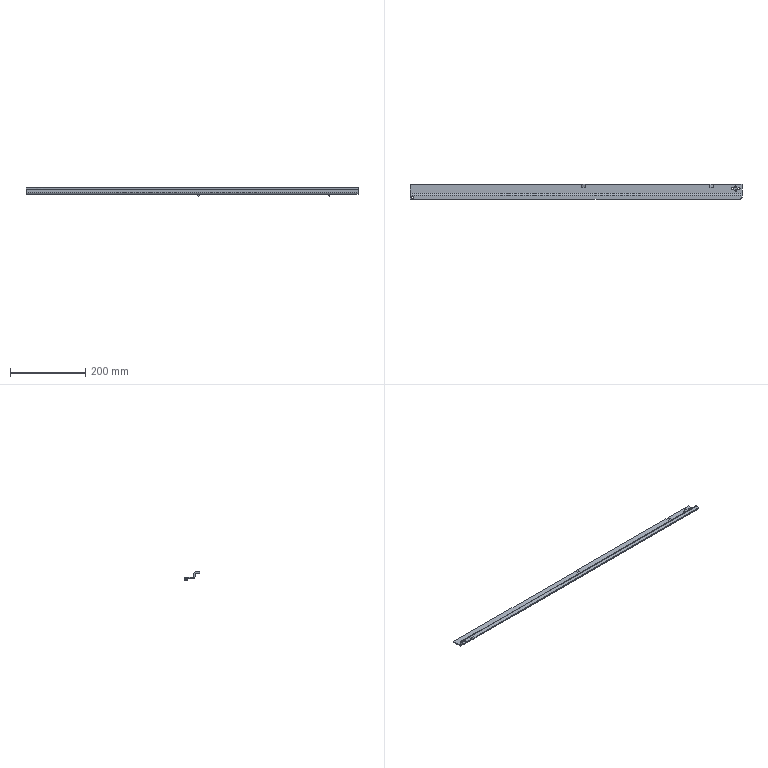Part | SolidWorks | features ICE 3, EdgeFlange 2, FormToolInstance 2, SMBaseFlange 2, Fillet 1, FlatPattern 1, SheetMetal 1 | 1 solid | 54 faces | box 880 x 40 x 21.683 mm | volume 132774 mm3 | plane 38 | cylinder 16 | commonest cylinder face diameters 6 x6 4 x4 3 x2 9 x2 10 x1 79.402 x1
STEP:
#1=CARTESIAN_POINT('',(10.,-6.,14.));
#2=VERTEX_POINT('',#1);
#3=CARTESIAN_POINT('',(4.,-6.,14.));
#4=VERTEX_POINT('',#3);
#5=CARTESIAN_POINT('',(7.,-6.,14.));
#6=DIRECTION('',(0.,0.,-1.));
#7=DIRECTION('',(-1.,0.,0.));
#8=AXIS2_PLACEMENT_3D('',#5,#6,#7);
#9=CIRCLE('',#8,3.);
#10=EDGE_CURVE('',#2,#4,#9,.T.);
#11=ORIENTED_EDGE('',*,*,#10,.F.);
#12=CARTESIAN_POINT('',(10.,-6.,11.));
#13=VERTEX_POINT('',#12);
#14=CARTESIAN_POINT('',(10.,-6.,14.));
#15=DIRECTION('',(0.,0.,-1.));
#16=VECTOR('',#15,1000.);
#17=LINE('',#14,#16);
#18=EDGE_CURVE('',#2,#13,#17,.T.);
#19=ORIENTED_EDGE('',*,*,#18,.T.);
#20=CARTESIAN_POINT('',(4.,-6.,11.));
#21=VERTEX_POINT('',#20);
#22=CARTESIAN_POINT('',(7.,-6.,11.));
#23=DIRECTION('',(0.,0.,-1.));
#24=DIRECTION('',(-1.,0.,0.));
#25=AXIS2_PLACEMENT_3D('',#22,#23,#24);
#26=CIRCLE('',#25,3.);
#27=EDGE_CURVE('',#13,#21,#26,.T.);
#28=ORIENTED_EDGE('',*,*,#27,.T.);
#29=CARTESIAN_POINT('',(4.,-6.,14.));
#30=DIRECTION('',(0.,0.,-1.));
#31=VECTOR('',#30,1000.);
#32=LINE('',#29,#31);
#33=EDGE_CURVE('',#4,#21,#32,.T.);
#34=ORIENTED_EDGE('',*,*,#33,.F.);
#35=EDGE_LOOP('',(#11,#19,#28,#34));
#36=FACE_OUTER_BOUND('',#35,.T.);
#37=CARTESIAN_POINT('',(7.,-6.,14.));
#38=DIRECTION('',(0.,0.,-1.));
#39=DIRECTION('',(-1.,0.,0.));
#40=AXIS2_PLACEMENT_3D('',#37,#38,#39);
#41=CYLINDRICAL_SURFACE('',#40,3.);
#42=ADVANCED_FACE('',(#36),#41,.F.);
#43=CARTESIAN_POINT('',(865.,22.,0.));
#44=VERTEX_POINT('',#43);
#45=CARTESIAN_POINT('',(861.,22.,0.));
#46=VERTEX_POINT('',#45);
#47=CARTESIAN_POINT('',(863.,22.,0.));
#48=DIRECTION('',(0.,0.,-1.));
#49=DIRECTION('',(-1.,0.,0.));
#50=AXIS2_PLACEMENT_3D('',#47,#48,#49);
#51=CIRCLE('',#50,2.);
#52=EDGE_CURVE('',#44,#46,#51,.T.);
#53=ORIENTED_EDGE('',*,*,#52,.F.);
#54=CARTESIAN_POINT('',(865.,22.,-3.));
#55=VERTEX_POINT('',#54);
#56=CARTESIAN_POINT('',(865.,22.,0.));
#57=DIRECTION('',(0.,0.,-1.));
#58=VECTOR('',#57,1000.);
#59=LINE('',#56,#58);
#60=EDGE_CURVE('',#44,#55,#59,.T.);
#61=ORIENTED_EDGE('',*,*,#60,.T.);
#62=CARTESIAN_POINT('',(861.,22.,-3.));
#63=VERTEX_POINT('',#62);
#64=CARTESIAN_POINT('',(863.,22.,-3.));
#65=DIRECTION('',(0.,0.,-1.));
#66=DIRECTION('',(-1.,0.,0.));
#67=AXIS2_PLACEMENT_3D('',#64,#65,#66);
#68=CIRCLE('',#67,2.);
#69=EDGE_CURVE('',#55,#63,#68,.T.);
#70=ORIENTED_EDGE('',*,*,#69,.T.);
#71=CARTESIAN_POINT('',(861.,22.,0.));
#72=DIRECTION('',(0.,0.,-1.));
#73=VECTOR('',#72,1000.);
#74=LINE('',#71,#73);
#75=EDGE_CURVE('',#46,#63,#74,.T.);
#76=ORIENTED_EDGE('',*,*,#75,.F.);
#77=EDGE_LOOP('',(#53,#61,#70,#76));
#78=FACE_OUTER_BOUND('',#77,.T.);
#79=CARTESIAN_POINT('',(863.,22.,0.));
#80=DIRECTION('',(0.,0.,-1.));
#81=DIRECTION('',(-1.,0.,0.));
#82=AXIS2_PLACEMENT_3D('',#79,#80,#81);
#83=CYLINDRICAL_SURFACE('',#82,2.);
#84=ADVANCED_FACE('',(#78),#83,.F.);
#85=CARTESIAN_POINT('',(865.,12.,0.));
#86=VERTEX_POINT('',#85);
#87=CARTESIAN_POINT('',(861.,12.,0.));
#88=VERTEX_POINT('',#87);
#89=CARTESIAN_POINT('',(863.,12.,0.));
#90=DIRECTION('',(0.,0.,-1.));
#91=DIRECTION('',(-1.,0.,0.));
#92=AXIS2_PLACEMENT_3D('',#89,#90,#91);
#93=CIRCLE('',#92,2.);
#94=EDGE_CURVE('',#86,#88,#93,.T.);
#95=ORIENTED_EDGE('',*,*,#94,.F.);
#96=CARTESIAN_POINT('',(865.,12.,-3.));
#97=VERTEX_POINT('',#96);
#98=CARTESIAN_POINT('',(865.,12.,0.));
#99=DIRECTION('',(0.,0.,-1.));
#100=VECTOR('',#99,1000.);
#101=LINE('',#98,#100);
#102=EDGE_CURVE('',#86,#97,#101,.T.);
#103=ORIENTED_EDGE('',*,*,#102,.T.);
#104=CARTESIAN_POINT('',(861.,12.,-3.));
#105=VERTEX_POINT('',#104);
#106=CARTESIAN_POINT('',(863.,12.,-3.));
#107=DIRECTION('',(0.,0.,-1.));
#108=DIRECTION('',(-1.,0.,0.));
#109=AXIS2_PLACEMENT_3D('',#106,#107,#108);
#110=CIRCLE('',#109,2.);
#111=EDGE_CURVE('',#97,#105,#110,.T.);
#112=ORIENTED_EDGE('',*,*,#111,.T.);
#113=CARTESIAN_POINT('',(861.,12.,0.));
#114=DIRECTION('',(0.,0.,-1.));
#115=VECTOR('',#114,1000.);
#116=LINE('',#113,#115);
#117=EDGE_CURVE('',#88,#105,#116,.T.);
#118=ORIENTED_EDGE('',*,*,#117,.F.);
#119=EDGE_LOOP('',(#95,#103,#112,#118));
#120=FACE_OUTER_BOUND('',#119,.T.);
#121=CARTESIAN_POINT('',(863.,12.,0.));
#122=DIRECTION('',(0.,0.,-1.));
#123=DIRECTION('',(-1.,0.,0.));
#124=AXIS2_PLACEMENT_3D('',#121,#122,#123);
#125=CYLINDRICAL_SURFACE('',#124,2.);
#126=ADVANCED_FACE('',(#120),#125,.F.);
#127=CARTESIAN_POINT('',(875.,17.,0.));
#128=VERTEX_POINT('',#127);
#129=CARTESIAN_POINT('',(869.,17.,0.));
#130=VERTEX_POINT('',#129);
#131=CARTESIAN_POINT('',(872.,17.,0.));
#132=DIRECTION('',(0.,0.,-1.));
#133=DIRECTION('',(-1.,0.,0.));
#134=AXIS2_PLACEMENT_3D('',#131,#132,#133);
#135=CIRCLE('',#134,3.);
#136=EDGE_CURVE('',#128,#130,#135,.T.);
#137=ORIENTED_EDGE('',*,*,#136,.F.);
#138=CARTESIAN_POINT('',(875.,17.,-3.));
#139=VERTEX_POINT('',#138);
#140=CARTESIAN_POINT('',(875.,17.,0.));
#141=DIRECTION('',(0.,0.,-1.));
#142=VECTOR('',#141,1000.);
#143=LINE('',#140,#142);
#144=EDGE_CURVE('',#128,#139,#143,.T.);
#145=ORIENTED_EDGE('',*,*,#144,.T.);
#146=CARTESIAN_POINT('',(869.,17.,-3.));
#147=VERTEX_POINT('',#146);
#148=CARTESIAN_POINT('',(872.,17.,-3.));
#149=DIRECTION('',(0.,0.,-1.));
#150=DIRECTION('',(-1.,0.,0.));
#151=AXIS2_PLACEMENT_3D('',#148,#149,#150);
#152=CIRCLE('',#151,3.);
#153=EDGE_CURVE('',#139,#147,#152,.T.);
#154=ORIENTED_EDGE('',*,*,#153,.T.);
#155=CARTESIAN_POINT('',(869.,17.,0.));
#156=DIRECTION('',(0.,0.,-1.));
#157=VECTOR('',#156,1000.);
#158=LINE('',#155,#157);
#159=EDGE_CURVE('',#130,#147,#158,.T.);
#160=ORIENTED_EDGE('',*,*,#159,.F.);
#161=EDGE_LOOP('',(#137,#145,#154,#160));
#162=FACE_OUTER_BOUND('',#161,.T.);
#163=CARTESIAN_POINT('',(872.,17.,0.));
#164=DIRECTION('',(0.,0.,-1.));
#165=DIRECTION('',(-1.,0.,0.));
#166=AXIS2_PLACEMENT_3D('',#163,#164,#165);
#167=CYLINDRICAL_SURFACE('',#166,3.);
#168=ADVANCED_FACE('',(#162),#167,.F.);
#169=CARTESIAN_POINT('',(857.,17.,0.));
#170=VERTEX_POINT('',#169);
#171=CARTESIAN_POINT('',(851.,17.,0.));
#172=VERTEX_POINT('',#171);
#173=CARTESIAN_POINT('',(854.,17.,0.));
#174=DIRECTION('',(0.,0.,-1.));
#175=DIRECTION('',(-1.,0.,0.));
#176=AXIS2_PLACEMENT_3D('',#173,#174,#175);
#177=CIRCLE('',#176,3.);
#178=EDGE_CURVE('',#170,#172,#177,.T.);
#179=ORIENTED_EDGE('',*,*,#178,.F.);
#180=CARTESIAN_POINT('',(857.,17.,-3.));
#181=VERTEX_POINT('',#180);
#182=CARTESIAN_POINT('',(857.,17.,0.));
#183=DIRECTION('',(0.,0.,-1.));
#184=VECTOR('',#183,1000.);
#185=LINE('',#182,#184);
#186=EDGE_CURVE('',#170,#181,#185,.T.);
#187=ORIENTED_EDGE('',*,*,#186,.T.);
#188=CARTESIAN_POINT('',(851.,17.,-3.));
#189=VERTEX_POINT('',#188);
#190=CARTESIAN_POINT('',(854.,17.,-3.));
#191=DIRECTION('',(0.,0.,-1.));
#192=DIRECTION('',(-1.,0.,0.));
#193=AXIS2_PLACEMENT_3D('',#190,#191,#192);
#194=CIRCLE('',#193,3.);
#195=EDGE_CURVE('',#181,#189,#194,.T.);
#196=ORIENTED_EDGE('',*,*,#195,.T.);
#197=CARTESIAN_POINT('',(851.,17.,0.));
#198=DIRECTION('',(0.,0.,-1.));
#199=VECTOR('',#198,1000.);
#200=LINE('',#197,#199);
#201=EDGE_CURVE('',#172,#189,#200,.T.);
#202=ORIENTED_EDGE('',*,*,#201,.F.);
#203=EDGE_LOOP('',(#179,#187,#196,#202));
#204=FACE_OUTER_BOUND('',#203,.T.);
#205=CARTESIAN_POINT('',(854.,17.,0.));
#206=DIRECTION('',(0.,0.,-1.));
#207=DIRECTION('',(-1.,0.,0.));
#208=AXIS2_PLACEMENT_3D('',#205,#206,#207);
#209=CYLINDRICAL_SURFACE('',#208,3.);
#210=ADVANCED_FACE('',(#204),#209,.F.);
#211=CARTESIAN_POINT('',(44.709,-11.,11.));
#212=VERTEX_POINT('',#211);
#213=CARTESIAN_POINT('',(44.709,-11.,14.));
#214=VERTEX_POINT('',#213);
#215=CARTESIAN_POINT('',(44.709,-11.,11.));
#216=DIRECTION('',(0.,0.,1.));
#217=VECTOR('',#216,1000.);
#218=LINE('',#215,#217);
#219=EDGE_CURVE('',#212,#214,#218,.T.);
#220=ORIENTED_EDGE('',*,*,#219,.F.);
#221=CARTESIAN_POINT('',(875.,-11.,11.));
#222=VERTEX_POINT('',#221);
#223=CARTESIAN_POINT('',(0.,-11.,11.));
#224=DIRECTION('',(-1.,0.,0.));
#225=VECTOR('',#224,1000.);
#226=LINE('',#223,#225);
#227=EDGE_CURVE('',#222,#212,#226,.T.);
#228=ORIENTED_EDGE('',*,*,#227,.F.);
#229=CARTESIAN_POINT('',(875.,-11.,14.));
#230=VERTEX_POINT('',#229);
#231=CARTESIAN_POINT('',(875.,-11.,14.));
#232=DIRECTION('',(0.,0.,1.));
#233=VECTOR('',#232,1000.);
#234=LINE('',#231,#233);
#235=EDGE_CURVE('',#222,#230,#234,.T.);
#236=ORIENTED_EDGE('',*,*,#235,.T.);
#237=CARTESIAN_POINT('',(0.,-11.,14.));
#238=DIRECTION('',(-1.,0.,0.));
#239=VECTOR('',#238,1000.);
#240=LINE('',#237,#239);
#241=EDGE_CURVE('',#230,#214,#240,.T.);
#242=ORIENTED_EDGE('',*,*,#241,.T.);
#243=EDGE_LOOP('',(#220,#228,#236,#242));
#244=FACE_OUTER_BOUND('',#243,.T.);
#245=CARTESIAN_POINT('',(0.,-11.,14.));
#246=DIRECTION('',(0.,-1.,0.));
#247=DIRECTION('',(0.,0.,-1.));
#248=AXIS2_PLACEMENT_3D('',#245,#246,#247);
#249=PLANE('',#248);
#250=ADVANCED_FACE('',(#244),#249,.T.);
#251=CARTESIAN_POINT('',(863.,22.,-3.));
#252=DIRECTION('',(0.,0.,-1.));
#253=DIRECTION('',(-1.,0.,0.));
#254=AXIS2_PLACEMENT_3D('',#251,#252,#253);
#255=CIRCLE('',#254,2.);
#256=EDGE_CURVE('',#63,#55,#255,.T.);
#257=ORIENTED_EDGE('',*,*,#256,.F.);
#258=ORIENTED_EDGE('',*,*,#69,.F.);
#259=EDGE_LOOP('',(#257,#258));
#260=FACE_BOUND('',#259,.T.);
#261=CARTESIAN_POINT('',(863.,12.,-3.));
#262=DIRECTION('',(0.,0.,-1.));
#263=DIRECTION('',(-1.,0.,0.));
#264=AXIS2_PLACEMENT_3D('',#261,#262,#263);
#265=CIRCLE('',#264,2.);
#266=EDGE_CURVE('',#105,#97,#265,.T.);
#267=ORIENTED_EDGE('',*,*,#266,.F.);
#268=ORIENTED_EDGE('',*,*,#111,.F.);
#269=EDGE_LOOP('',(#267,#268));
#270=FACE_BOUND('',#269,.T.);
#271=CARTESIAN_POINT('',(872.,17.,-3.));
#272=DIRECTION('',(0.,0.,-1.));
#273=DIRECTION('',(-1.,0.,0.));
#274=AXIS2_PLACEMENT_3D('',#271,#272,#273);
#275=CIRCLE('',#274,3.);
#276=EDGE_CURVE('',#147,#139,#275,.T.);
#277=ORIENTED_EDGE('',*,*,#276,.F.);
#278=ORIENTED_EDGE('',*,*,#153,.F.);
#279=EDGE_LOOP('',(#277,#278));
#280=FACE_BOUND('',#279,.T.);
#281=CARTESIAN_POINT('',(854.,17.,-3.));
#282=DIRECTION('',(0.,0.,-1.));
#283=DIRECTION('',(-1.,0.,0.));
#284=AXIS2_PLACEMENT_3D('',#281,#282,#283);
#285=CIRCLE('',#284,3.);
#286=EDGE_CURVE('',#189,#181,#285,.T.);
#287=ORIENTED_EDGE('',*,*,#286,.F.);
#288=ORIENTED_EDGE('',*,*,#195,.F.);
#289=EDGE_LOOP('',(#287,#288));
#290=FACE_BOUND('',#289,.T.);
#291=CARTESIAN_POINT('',(455.,20.,-3.));
#292=VERTEX_POINT('',#291);
#293=CARTESIAN_POINT('',(459.,20.,-3.));
#294=VERTEX_POINT('',#293);
#295=CARTESIAN_POINT('',(0.,20.,-3.));
#296=DIRECTION('',(1.,0.,0.));
#297=VECTOR('',#296,1000.);
#298=LINE('',#295,#297);
#299=EDGE_CURVE('',#292,#294,#298,.T.);
#300=ORIENTED_EDGE('',*,*,#299,.T.);
#301=CARTESIAN_POINT('',(465.708,20.,-3.));
#302=VERTEX_POINT('',#301);
#303=CARTESIAN_POINT('',(0.,20.,-3.));
#304=DIRECTION('',(1.,0.,0.));
#305=VECTOR('',#304,1000.);
#306=LINE('',#303,#305);
#307=EDGE_CURVE('',#294,#302,#306,.T.);
#308=ORIENTED_EDGE('',*,*,#307,.T.);
#309=CARTESIAN_POINT('',(465.708,28.,-3.));
#310=VERTEX_POINT('',#309);
#311=CARTESIAN_POINT('',(465.708,28.,-3.));
#312=DIRECTION('',(0.,-1.,0.));
#313=VECTOR('',#312,1000.);
#314=LINE('',#311,#313);
#315=EDGE_CURVE('',#310,#302,#314,.T.);
#316=ORIENTED_EDGE('',*,*,#315,.F.);
#317=CARTESIAN_POINT('',(794.292,28.,-3.));
#318=VERTEX_POINT('',#317);
#319=CARTESIAN_POINT('',(0.,28.,-3.));
#320=DIRECTION('',(-1.,0.,0.));
#321=VECTOR('',#320,1000.);
#322=LINE('',#319,#321);
#323=EDGE_CURVE('',#318,#310,#322,.T.);
#324=ORIENTED_EDGE('',*,*,#323,.F.);
#325=CARTESIAN_POINT('',(794.292,20.,-3.));
#326=VERTEX_POINT('',#325);
#327=CARTESIAN_POINT('',(794.292,28.,-3.));
#328=DIRECTION('',(0.,1.,0.));
#329=VECTOR('',#328,1000.);
#330=LINE('',#327,#329);
#331=EDGE_CURVE('',#326,#318,#330,.T.);
#332=ORIENTED_EDGE('',*,*,#331,.F.);
#333=CARTESIAN_POINT('',(801.,20.,-3.));
#334=VERTEX_POINT('',#333);
#335=CARTESIAN_POINT('',(0.,20.,-3.));
#336=DIRECTION('',(1.,0.,0.));
#337=VECTOR('',#336,1000.);
#338=LINE('',#335,#337);
#339=EDGE_CURVE('',#326,#334,#338,.T.);
#340=ORIENTED_EDGE('',*,*,#339,.T.);
#341=CARTESIAN_POINT('',(805.,20.,-3.));
#342=VERTEX_POINT('',#341);
#343=CARTESIAN_POINT('',(0.,20.,-3.));
#344=DIRECTION('',(-1.,0.,0.));
#345=VECTOR('',#344,1000.);
#346=LINE('',#343,#345);
#347=EDGE_CURVE('',#342,#334,#346,.T.);
#348=ORIENTED_EDGE('',*,*,#347,.F.);
#349=CARTESIAN_POINT('',(805.,28.,-3.));
#350=VERTEX_POINT('',#349);
#351=CARTESIAN_POINT('',(805.,28.,-3.));
#352=DIRECTION('',(0.,-1.,0.));
#353=VECTOR('',#352,1000.);
#354=LINE('',#351,#353);
#355=EDGE_CURVE('',#350,#342,#354,.T.);
#356=ORIENTED_EDGE('',*,*,#355,.F.);
#357=CARTESIAN_POINT('',(880.,28.,-3.));
#358=VERTEX_POINT('',#357);
#359=CARTESIAN_POINT('',(0.,28.,-3.));
#360=DIRECTION('',(-1.,0.,0.));
#361=VECTOR('',#360,1000.);
#362=LINE('',#359,#361);
#363=EDGE_CURVE('',#358,#350,#362,.T.);
#364=ORIENTED_EDGE('',*,*,#363,.F.);
#365=CARTESIAN_POINT('',(880.,4.5,-3.));
#366=VERTEX_POINT('',#365);
#367=CARTESIAN_POINT('',(880.,0.,-3.));
#368=DIRECTION('',(0.,1.,0.));
#369=VECTOR('',#368,1000.);
#370=LINE('',#367,#369);
#371=EDGE_CURVE('',#366,#358,#370,.T.);
#372=ORIENTED_EDGE('',*,*,#371,.F.);
#373=CARTESIAN_POINT('',(0.,4.5,-3.));
#374=VERTEX_POINT('',#373);
#375=CARTESIAN_POINT('',(880.,4.5,-3.));
#376=DIRECTION('',(-1.,0.,0.));
#377=VECTOR('',#376,1000.);
#378=LINE('',#375,#377);
#379=EDGE_CURVE('',#366,#374,#378,.T.);
#380=ORIENTED_EDGE('',*,*,#379,.T.);
#381=CARTESIAN_POINT('',(0.,28.,-3.));
#382=VERTEX_POINT('',#381);
#383=CARTESIAN_POINT('',(0.,0.,-3.));
#384=DIRECTION('',(0.,-1.,0.));
#385=VECTOR('',#384,1000.);
#386=LINE('',#383,#385);
#387=EDGE_CURVE('',#382,#374,#386,.T.);
#388=ORIENTED_EDGE('',*,*,#387,.F.);
#389=CARTESIAN_POINT('',(455.,28.,-3.));
#390=VERTEX_POINT('',#389);
#391=CARTESIAN_POINT('',(0.,28.,-3.));
#392=DIRECTION('',(-1.,0.,0.));
#393=VECTOR('',#392,1000.);
#394=LINE('',#391,#393);
#395=EDGE_CURVE('',#390,#382,#394,.T.);
#396=ORIENTED_EDGE('',*,*,#395,.F.);
#397=CARTESIAN_POINT('',(455.,28.,-3.));
#398=DIRECTION('',(0.,1.,0.));
#399=VECTOR('',#398,1000.);
#400=LINE('',#397,#399);
#401=EDGE_CURVE('',#292,#390,#400,.T.);
#402=ORIENTED_EDGE('',*,*,#401,.F.);
#403=EDGE_LOOP('',(#300,#308,#316,#324,#332,#340,#348,#356,#364,#372,#380,#388,#396,#402));
#404=FACE_OUTER_BOUND('',#403,.T.);
#405=CARTESIAN_POINT('',(0.,28.,-3.));
#406=DIRECTION('',(0.,0.,-1.));
#407=DIRECTION('',(-1.,0.,0.));
#408=AXIS2_PLACEMENT_3D('',#405,#406,#407);
#409=PLANE('',#408);
#410=ADVANCED_FACE('',(#260,#270,#280,#290,#404),#409,.T.);
#411=CARTESIAN_POINT('',(455.,28.,0.));
#412=VERTEX_POINT('',#411);
#413=CARTESIAN_POINT('',(455.,28.,-3.));
#414=DIRECTION('',(0.,0.,1.));
#415=VECTOR('',#414,1000.);
#416=LINE('',#413,#415);
#417=EDGE_CURVE('',#390,#412,#416,.T.);
#418=ORIENTED_EDGE('',*,*,#417,.F.);
#419=ORIENTED_EDGE('',*,*,#395,.T.);
#420=CARTESIAN_POINT('',(0.,28.,0.));
#421=VERTEX_POINT('',#420);
#422=CARTESIAN_POINT('',(0.,28.,-3.));
#423=DIRECTION('',(0.,0.,1.));
#424=VECTOR('',#423,1000.);
#425=LINE('',#422,#424);
#426=EDGE_CURVE('',#382,#421,#425,.T.);
#427=ORIENTED_EDGE('',*,*,#426,.T.);
#428=CARTESIAN_POINT('',(0.,28.,0.));
#429=DIRECTION('',(-1.,0.,0.));
#430=VECTOR('',#429,1000.);
#431=LINE('',#428,#430);
#432=EDGE_CURVE('',#412,#421,#431,.T.);
#433=ORIENTED_EDGE('',*,*,#432,.F.);
#434=EDGE_LOOP('',(#418,#419,#427,#433));
#435=FACE_OUTER_BOUND('',#434,.T.);
#436=CARTESIAN_POINT('',(0.,28.,-3.));
#437=DIRECTION('',(0.,1.,0.));
#438=DIRECTION('',(0.,0.,1.));
#439=AXIS2_PLACEMENT_3D('',#436,#437,#438);
#440=PLANE('',#439);
#441=ADVANCED_FACE('',(#435),#440,.T.);
#442=CARTESIAN_POINT('',(805.,28.,0.));
#443=VERTEX_POINT('',#442);
#444=CARTESIAN_POINT('',(805.,28.,-3.));
#445=DIRECTION('',(0.,0.,-1.));
#446=VECTOR('',#445,1000.);
#447=LINE('',#444,#446);
#448=EDGE_CURVE('',#443,#350,#447,.T.);
#449=ORIENTED_EDGE('',*,*,#448,.F.);
#450=CARTESIAN_POINT('',(880.,28.,0.));
#451=VERTEX_POINT('',#450);
#452=CARTESIAN_POINT('',(0.,28.,0.));
#453=DIRECTION('',(-1.,0.,0.));
#454=VECTOR('',#453,1000.);
#455=LINE('',#452,#454);
#456=EDGE_CURVE('',#451,#443,#455,.T.);
#457=ORIENTED_EDGE('',*,*,#456,.F.);
#458=CARTESIAN_POINT('',(880.,28.,-3.));
#459=DIRECTION('',(0.,0.,1.));
#460=VECTOR('',#459,1000.);
#461=LINE('',#458,#460);
#462=EDGE_CURVE('',#358,#451,#461,.T.);
#463=ORIENTED_EDGE('',*,*,#462,.F.);
#464=ORIENTED_EDGE('',*,*,#363,.T.);
#465=EDGE_LOOP('',(#449,#457,#463,#464));
#466=FACE_OUTER_BOUND('',#465,.T.);
#467=CARTESIAN_POINT('',(0.,28.,-3.));
#468=DIRECTION('',(0.,1.,0.));
#469=DIRECTION('',(0.,0.,1.));
#470=AXIS2_PLACEMENT_3D('',#467,#468,#469);
#471=PLANE('',#470);
#472=ADVANCED_FACE('',(#466),#471,.T.);
#473=CARTESIAN_POINT('',(0.,0.,1.5));
#474=VERTEX_POINT('',#473);
#475=CARTESIAN_POINT('',(0.,0.,9.5));
#476=VERTEX_POINT('',#475);
#477=CARTESIAN_POINT('',(0.,0.,11.));
#478=DIRECTION('',(0.,0.,1.));
#479=VECTOR('',#478,1000.);
#480=LINE('',#477,#479);
#481=EDGE_CURVE('',#474,#476,#480,.T.);
#482=ORIENTED_EDGE('',*,*,#481,.T.);
#483=CARTESIAN_POINT('',(0.,3.,9.5));
#484=VERTEX_POINT('',#483);
#485=CARTESIAN_POINT('',(0.,0.,9.5));
#486=DIRECTION('',(0.,1.,0.));
#487=VECTOR('',#486,1000.);
#488=LINE('',#485,#487);
#489=EDGE_CURVE('',#476,#484,#488,.T.);
#490=ORIENTED_EDGE('',*,*,#489,.T.);
#491=CARTESIAN_POINT('',(0.,3.,1.5));
#492=VERTEX_POINT('',#491);
#493=CARTESIAN_POINT('',(0.,3.,0.));
#494=DIRECTION('',(0.,0.,1.));
#495=VECTOR('',#494,1000.);
#496=LINE('',#493,#495);
#497=EDGE_CURVE('',#492,#484,#496,.T.);
#498=ORIENTED_EDGE('',*,*,#497,.F.);
#499=CARTESIAN_POINT('',(0.,0.,1.5));
#500=DIRECTION('',(0.,-1.,0.));
#501=VECTOR('',#500,1000.);
#502=LINE('',#499,#501);
#503=EDGE_CURVE('',#492,#474,#502,.T.);
#504=ORIENTED_EDGE('',*,*,#503,.T.);
#505=EDGE_LOOP('',(#482,#490,#498,#504));
#506=FACE_OUTER_BOUND('',#505,.T.);
#507=CARTESIAN_POINT('',(0.,0.,11.));
#508=DIRECTION('',(-1.,0.,0.));
#509=DIRECTION('',(0.,0.,1.));
#510=AXIS2_PLACEMENT_3D('',#507,#508,#509);
#511=PLANE('',#510);
#512=ADVANCED_FACE('',(#506),#511,.T.);
#513=CARTESIAN_POINT('',(880.,0.,9.5));
#514=VERTEX_POINT('',#513);
#515=CARTESIAN_POINT('',(880.,0.,1.5));
#516=VERTEX_POINT('',#515);
#517=CARTESIAN_POINT('',(880.,0.,0.));
#518=DIRECTION('',(0.,0.,-1.));
#519=VECTOR('',#518,1000.);
#520=LINE('',#517,#519);
#521=EDGE_CURVE('',#514,#516,#520,.T.);
#522=ORIENTED_EDGE('',*,*,#521,.F.);
#523=CARTESIAN_POINT('',(0.,0.,9.5));
#524=DIRECTION('',(1.,0.,0.));
#525=VECTOR('',#524,1000.);
#526=LINE('',#523,#525);
#527=EDGE_CURVE('',#476,#514,#526,.T.);
#528=ORIENTED_EDGE('',*,*,#527,.F.);
#529=ORIENTED_EDGE('',*,*,#481,.F.);
#530=CARTESIAN_POINT('',(880.,0.,1.5));
#531=DIRECTION('',(1.,0.,0.));
#532=VECTOR('',#531,1000.);
#533=LINE('',#530,#532);
#534=EDGE_CURVE('',#474,#516,#533,.T.);
#535=ORIENTED_EDGE('',*,*,#534,.T.);
#536=EDGE_LOOP('',(#522,#528,#529,#535));
#537=FACE_OUTER_BOUND('',#536,.T.);
#538=CARTESIAN_POINT('',(880.,0.,0.));
#539=DIRECTION('',(0.,-1.,0.));
#540=DIRECTION('',(0.,0.,-1.));
#541=AXIS2_PLACEMENT_3D('',#538,#539,#540);
#542=PLANE('',#541);
#543=ADVANCED_FACE('',(#537),#542,.T.);
#544=CARTESIAN_POINT('',(880.,3.,9.5));
#545=VERTEX_POINT('',#544);
#546=CARTESIAN_POINT('',(0.,3.,9.5));
#547=DIRECTION('',(1.,0.,0.));
#548=VECTOR('',#547,1000.);
#549=LINE('',#546,#548);
#550=EDGE_CURVE('',#484,#545,#549,.T.);
#551=ORIENTED_EDGE('',*,*,#550,.T.);
#552=CARTESIAN_POINT('',(880.,3.,1.5));
#553=VERTEX_POINT('',#552);
#554=CARTESIAN_POINT('',(880.,3.,0.));
#555=DIRECTION('',(0.,0.,-1.));
#556=VECTOR('',#555,1000.);
#557=LINE('',#554,#556);
#558=EDGE_CURVE('',#545,#553,#557,.T.);
#559=ORIENTED_EDGE('',*,*,#558,.T.);
#560=CARTESIAN_POINT('',(0.,3.,1.5));
#561=DIRECTION('',(1.,0.,0.));
#562=VECTOR('',#561,1000.);
#563=LINE('',#560,#562);
#564=EDGE_CURVE('',#492,#553,#563,.T.);
#565=ORIENTED_EDGE('',*,*,#564,.F.);
#566=ORIENTED_EDGE('',*,*,#497,.T.);
#567=EDGE_LOOP('',(#551,#559,#565,#566));
#568=FACE_OUTER_BOUND('',#567,.T.);
#569=CARTESIAN_POINT('',(880.,3.,0.));
#570=DIRECTION('',(0.,-1.,0.));
#571=DIRECTION('',(0.,0.,-1.));
#572=AXIS2_PLACEMENT_3D('',#569,#570,#571);
#573=PLANE('',#572);
#574=ADVANCED_FACE('',(#568),#573,.F.);
#575=CARTESIAN_POINT('',(880.,4.5,0.));
#576=VERTEX_POINT('',#575);
#577=CARTESIAN_POINT('',(880.,0.,0.));
#578=DIRECTION('',(0.,1.,0.));
#579=VECTOR('',#578,1000.);
#580=LINE('',#577,#579);
#581=EDGE_CURVE('',#576,#451,#580,.T.);
#582=ORIENTED_EDGE('',*,*,#581,.F.);
#583=CARTESIAN_POINT('',(880.,4.5,0.));
#584=DIRECTION('',(0.,0.,-1.));
#585=VECTOR('',#584,1000.);
#586=LINE('',#583,#585);
#587=EDGE_CURVE('',#576,#366,#586,.T.);
#588=ORIENTED_EDGE('',*,*,#587,.T.);
#589=ORIENTED_EDGE('',*,*,#371,.T.);
#590=ORIENTED_EDGE('',*,*,#462,.T.);
#591=EDGE_LOOP('',(#582,#588,#589,#590));
#592=FACE_OUTER_BOUND('',#591,.T.);
#593=CARTESIAN_POINT('',(880.,0.,-3.));
#594=DIRECTION('',(1.,0.,0.));
#595=DIRECTION('',(0.,0.,-1.));
#596=AXIS2_PLACEMENT_3D('',#593,#594,#595);
#597=PLANE('',#596);
#598=ADVANCED_FACE('',(#592),#597,.T.);
#599=CARTESIAN_POINT('',(455.,20.,0.));
#600=VERTEX_POINT('',#599);
#601=CARTESIAN_POINT('',(465.,20.,0.));
#602=VERTEX_POINT('',#601);
#603=CARTESIAN_POINT('',(455.,20.,0.));
#604=DIRECTION('',(1.,0.,0.));
#605=VECTOR('',#604,1000.);
#606=LINE('',#603,#605);
#607=EDGE_CURVE('',#600,#602,#606,.T.);
#608=ORIENTED_EDGE('',*,*,#607,.F.);
#609=CARTESIAN_POINT('',(455.,20.,0.));
#610=DIRECTION('',(0.,1.,0.));
#611=VECTOR('',#610,1000.);
#612=LINE('',#609,#611);
#613=EDGE_CURVE('',#600,#412,#612,.T.);
#614=ORIENTED_EDGE('',*,*,#613,.T.);
#615=ORIENTED_EDGE('',*,*,#432,.T.);
#616=CARTESIAN_POINT('',(0.,4.5,0.));
#617=VERTEX_POINT('',#616);
#618=CARTESIAN_POINT('',(0.,0.,0.));
#619=DIRECTION('',(0.,-1.,0.));
#620=VECTOR('',#619,1000.);
#621=LINE('',#618,#620);
#622=EDGE_CURVE('',#421,#617,#621,.T.);
#623=ORIENTED_EDGE('',*,*,#622,.T.);
#624=CARTESIAN_POINT('',(880.,4.5,0.));
#625=DIRECTION('',(-1.,0.,0.));
#626=VECTOR('',#625,1000.);
#627=LINE('',#624,#626);
#628=EDGE_CURVE('',#576,#617,#627,.T.);
#629=ORIENTED_EDGE('',*,*,#628,.F.);
#630=ORIENTED_EDGE('',*,*,#581,.T.);
#631=ORIENTED_EDGE('',*,*,#456,.T.);
#632=CARTESIAN_POINT('',(805.,20.,0.));
#633=VERTEX_POINT('',#632);
#634=CARTESIAN_POINT('',(805.,28.,0.));
#635=DIRECTION('',(0.,-1.,0.));
#636=VECTOR('',#635,1000.);
#637=LINE('',#634,#636);
#638=EDGE_CURVE('',#443,#633,#637,.T.);
#639=ORIENTED_EDGE('',*,*,#638,.T.);
#640=CARTESIAN_POINT('',(795.,20.,0.));
#641=VERTEX_POINT('',#640);
#642=CARTESIAN_POINT('',(805.,20.,0.));
#643=DIRECTION('',(-1.,0.,0.));
#644=VECTOR('',#643,1000.);
#645=LINE('',#642,#644);
#646=EDGE_CURVE('',#633,#641,#645,.T.);
#647=ORIENTED_EDGE('',*,*,#646,.T.);
#648=CARTESIAN_POINT('',(795.,28.,0.));
#649=VERTEX_POINT('',#648);
#650=CARTESIAN_POINT('',(795.,28.,0.));
#651=DIRECTION('',(0.,-1.,0.));
#652=VECTOR('',#651,1000.);
#653=LINE('',#650,#652);
#654=EDGE_CURVE('',#649,#641,#653,.T.);
#655=ORIENTED_EDGE('',*,*,#654,.F.);
#656=CARTESIAN_POINT('',(465.,28.,0.));
#657=VERTEX_POINT('',#656);
#658=CARTESIAN_POINT('',(0.,28.,0.));
#659=DIRECTION('',(-1.,0.,0.));
#660=VECTOR('',#659,1000.);
#661=LINE('',#658,#660);
#662=EDGE_CURVE('',#649,#657,#661,.T.);
#663=ORIENTED_EDGE('',*,*,#662,.T.);
#664=CARTESIAN_POINT('',(465.,20.,0.));
#665=DIRECTION('',(0.,1.,0.));
#666=VECTOR('',#665,1000.);
#667=LINE('',#664,#666);
#668=EDGE_CURVE('',#602,#657,#667,.T.);
#669=ORIENTED_EDGE('',*,*,#668,.F.);
#670=EDGE_LOOP('',(#608,#614,#615,#623,#629,#630,#631,#639,#647,#655,#663,#669));
#671=FACE_OUTER_BOUND('',#670,.T.);
#672=CARTESIAN_POINT('',(863.,22.,0.));
#673=DIRECTION('',(0.,0.,-1.));
#674=DIRECTION('',(-1.,0.,0.));
#675=AXIS2_PLACEMENT_3D('',#672,#673,#674);
#676=CIRCLE('',#675,2.);
#677=EDGE_CURVE('',#46,#44,#676,.T.);
#678=ORIENTED_EDGE('',*,*,#677,.T.);
#679=ORIENTED_EDGE('',*,*,#52,.T.);
#680=EDGE_LOOP('',(#678,#679));
#681=FACE_BOUND('',#680,.T.);
#682=CARTESIAN_POINT('',(863.,12.,0.));
#683=DIRECTION('',(0.,0.,-1.));
#684=DIRECTION('',(-1.,0.,0.));
#685=AXIS2_PLACEMENT_3D('',#682,#683,#684);
#686=CIRCLE('',#685,2.);
#687=EDGE_CURVE('',#88,#86,#686,.T.);
#688=ORIENTED_EDGE('',*,*,#687,.T.);
#689=ORIENTED_EDGE('',*,*,#94,.T.);
#690=EDGE_LOOP('',(#688,#689));
#691=FACE_BOUND('',#690,.T.);
#692=CARTESIAN_POINT('',(872.,17.,0.));
#693=DIRECTION('',(0.,0.,-1.));
#694=DIRECTION('',(-1.,0.,0.));
#695=AXIS2_PLACEMENT_3D('',#692,#693,#694);
#696=CIRCLE('',#695,3.);
#697=EDGE_CURVE('',#130,#128,#696,.T.);
#698=ORIENTED_EDGE('',*,*,#697,.T.);
#699=ORIENTED_EDGE('',*,*,#136,.T.);
#700=EDGE_LOOP('',(#698,#699));
#701=FACE_BOUND('',#700,.T.);
#702=CARTESIAN_POINT('',(854.,17.,0.));
#703=DIRECTION('',(0.,0.,-1.));
#704=DIRECTION('',(-1.,0.,0.));
#705=AXIS2_PLACEMENT_3D('',#702,#703,#704);
#706=CIRCLE('',#705,3.);
#707=EDGE_CURVE('',#172,#170,#706,.T.);
#708=ORIENTED_EDGE('',*,*,#707,.T.);
#709=ORIENTED_EDGE('',*,*,#178,.T.);
#710=EDGE_LOOP('',(#708,#709));
#711=FACE_BOUND('',#710,.T.);
#712=CARTESIAN_POINT('',(0.,28.,0.));
#713=DIRECTION('',(0.,0.,-1.));
#714=DIRECTION('',(-1.,0.,0.));
#715=AXIS2_PLACEMENT_3D('',#712,#713,#714);
#716=PLANE('',#715);
#717=ADVANCED_FACE('',(#671,#681,#691,#701,#711),#716,.F.);
#718=CARTESIAN_POINT('',(0.,4.5,0.));
#719=DIRECTION('',(0.,0.,-1.));
#720=VECTOR('',#719,1000.);
#721=LINE('',#718,#720);
#722=EDGE_CURVE('',#617,#374,#721,.T.);
#723=ORIENTED_EDGE('',*,*,#722,.F.);
#724=ORIENTED_EDGE('',*,*,#622,.F.);
#725=ORIENTED_EDGE('',*,*,#426,.F.);
#726=ORIENTED_EDGE('',*,*,#387,.T.);
#727=EDGE_LOOP('',(#723,#724,#725,#726));
#728=FACE_OUTER_BOUND('',#727,.T.);
#729=CARTESIAN_POINT('',(0.,0.,-3.));
#730=DIRECTION('',(-1.,0.,0.));
#731=DIRECTION('',(0.,0.,1.));
#732=AXIS2_PLACEMENT_3D('',#729,#730,#731);
#733=PLANE('',#732);
#734=ADVANCED_FACE('',(#728),#733,.T.);
#735=CARTESIAN_POINT('',(455.,28.,-5.));
#736=VERTEX_POINT('',#735);
#737=CARTESIAN_POINT('',(465.,28.,0.));
#738=DIRECTION('',(-0.8944,0.,-0.4472));
#739=VECTOR('',#738,1000.);
#740=LINE('',#737,#739);
#741=EDGE_CURVE('',#657,#736,#740,.T.);
#742=ORIENTED_EDGE('',*,*,#741,.F.);
#743=ORIENTED_EDGE('',*,*,#662,.F.);
#744=CARTESIAN_POINT('',(805.,28.,-5.));
#745=VERTEX_POINT('',#744);
#746=CARTESIAN_POINT('',(795.,28.,0.));
#747=DIRECTION('',(0.8944,0.,-0.4472));
#748=VECTOR('',#747,1000.);
#749=LINE('',#746,#748);
#750=EDGE_CURVE('',#649,#745,#749,.T.);
#751=ORIENTED_EDGE('',*,*,#750,.T.);
#752=CARTESIAN_POINT('',(803.658,28.,-7.683));
#753=VERTEX_POINT('',#752);
#754=CARTESIAN_POINT('',(805.,28.,-5.));
#755=DIRECTION('',(0.4472,0.,0.8944));
#756=VECTOR('',#755,1000.);
#757=LINE('',#754,#756);
#758=EDGE_CURVE('',#753,#745,#757,.T.);
#759=ORIENTED_EDGE('',*,*,#758,.F.);
#760=CARTESIAN_POINT('',(793.658,28.,-2.683));
#761=DIRECTION('',(0.8944,0.,-0.4472));
#762=VECTOR('',#761,1000.);
#763=LINE('',#760,#762);
#764=EDGE_CURVE('',#318,#753,#763,.T.);
#765=ORIENTED_EDGE('',*,*,#764,.F.);
#766=ORIENTED_EDGE('',*,*,#323,.T.);
#767=CARTESIAN_POINT('',(456.342,28.,-7.683));
#768=VERTEX_POINT('',#767);
#769=CARTESIAN_POINT('',(466.342,28.,-2.683));
#770=DIRECTION('',(-0.8944,0.,-0.4472));
#771=VECTOR('',#770,1000.);
#772=LINE('',#769,#771);
#773=EDGE_CURVE('',#310,#768,#772,.T.);
#774=ORIENTED_EDGE('',*,*,#773,.T.);
#775=CARTESIAN_POINT('',(455.,28.,-5.));
#776=DIRECTION('',(-0.4472,0.,0.8944));
#777=VECTOR('',#776,1000.);
#778=LINE('',#775,#777);
#779=EDGE_CURVE('',#768,#736,#778,.T.);
#780=ORIENTED_EDGE('',*,*,#779,.T.);
#781=EDGE_LOOP('',(#742,#743,#751,#759,#765,#766,#774,#780));
#782=FACE_OUTER_BOUND('',#781,.T.);
#783=CARTESIAN_POINT('',(0.,28.,-3.));
#784=DIRECTION('',(0.,1.,0.));
#785=DIRECTION('',(0.,0.,1.));
#786=AXIS2_PLACEMENT_3D('',#783,#784,#785);
#787=PLANE('',#786);
#788=ADVANCED_FACE('',(#782),#787,.T.);
#789=ORIENTED_EDGE('',*,*,#503,.F.);
#790=CARTESIAN_POINT('',(0.,4.5,1.5));
#791=DIRECTION('',(-1.,0.,0.));
#792=DIRECTION('',(0.,0.,-1.));
#793=AXIS2_PLACEMENT_3D('',#790,#791,#792);
#794=CIRCLE('',#793,1.5);
#795=EDGE_CURVE('',#617,#492,#794,.T.);
#796=ORIENTED_EDGE('',*,*,#795,.F.);
#797=ORIENTED_EDGE('',*,*,#722,.T.);
#798=CARTESIAN_POINT('',(0.,4.5,1.5));
#799=DIRECTION('',(-1.,0.,0.));
#800=DIRECTION('',(0.,0.,-1.));
#801=AXIS2_PLACEMENT_3D('',#798,#799,#800);
#802=CIRCLE('',#801,4.5);
#803=EDGE_CURVE('',#374,#474,#802,.T.);
#804=ORIENTED_EDGE('',*,*,#803,.T.);
#805=EDGE_LOOP('',(#789,#796,#797,#804));
#806=FACE_OUTER_BOUND('',#805,.T.);
#807=CARTESIAN_POINT('',(0.,4.5,1.5));
#808=DIRECTION('',(-1.,0.,0.));
#809=DIRECTION('',(0.,0.,1.));
#810=AXIS2_PLACEMENT_3D('',#807,#808,#809);
#811=PLANE('',#810);
#812=ADVANCED_FACE('',(#806),#811,.T.);
#813=CARTESIAN_POINT('',(880.,4.5,1.5));
#814=DIRECTION('',(1.,0.,0.));
#815=DIRECTION('',(0.,0.,-1.));
#816=AXIS2_PLACEMENT_3D('',#813,#814,#815);
#817=CIRCLE('',#816,1.5);
#818=EDGE_CURVE('',#553,#576,#817,.T.);
#819=ORIENTED_EDGE('',*,*,#818,.F.);
#820=CARTESIAN_POINT('',(880.,3.,1.5));
#821=DIRECTION('',(0.,-1.,0.));
#822=VECTOR('',#821,1000.);
#823=LINE('',#820,#822);
#824=EDGE_CURVE('',#553,#516,#823,.T.);
#825=ORIENTED_EDGE('',*,*,#824,.T.);
#826=CARTESIAN_POINT('',(880.,4.5,1.5));
#827=DIRECTION('',(1.,0.,0.));
#828=DIRECTION('',(0.,0.,-1.));
#829=AXIS2_PLACEMENT_3D('',#826,#827,#828);
#830=CIRCLE('',#829,4.5);
#831=EDGE_CURVE('',#516,#366,#830,.T.);
#832=ORIENTED_EDGE('',*,*,#831,.T.);
#833=ORIENTED_EDGE('',*,*,#587,.F.);
#834=EDGE_LOOP('',(#819,#825,#832,#833));
#835=FACE_OUTER_BOUND('',#834,.T.);
#836=CARTESIAN_POINT('',(880.,4.5,1.5));
#837=DIRECTION('',(-1.,0.,0.));
#838=DIRECTION('',(0.,0.,1.));
#839=AXIS2_PLACEMENT_3D('',#836,#837,#838);
#840=PLANE('',#839);
#841=ADVANCED_FACE('',(#835),#840,.F.);
#842=ORIENTED_EDGE('',*,*,#379,.F.);
#843=ORIENTED_EDGE('',*,*,#831,.F.);
#844=ORIENTED_EDGE('',*,*,#534,.F.);
#845=ORIENTED_EDGE('',*,*,#803,.F.);
#846=EDGE_LOOP('',(#842,#843,#844,#845));
#847=FACE_OUTER_BOUND('',#846,.T.);
#848=CARTESIAN_POINT('',(880.,4.5,1.5));
#849=DIRECTION('',(1.,0.,0.));
#850=DIRECTION('',(0.,-1.,0.));
#851=AXIS2_PLACEMENT_3D('',#848,#849,#850);
#852=CYLINDRICAL_SURFACE('',#851,4.5);
#853=ADVANCED_FACE('',(#847),#852,.T.);
#854=ORIENTED_EDGE('',*,*,#628,.T.);
#855=ORIENTED_EDGE('',*,*,#795,.T.);
#856=ORIENTED_EDGE('',*,*,#564,.T.);
#857=ORIENTED_EDGE('',*,*,#818,.T.);
#858=EDGE_LOOP('',(#854,#855,#856,#857));
#859=FACE_OUTER_BOUND('',#858,.T.);
#860=CARTESIAN_POINT('',(880.,4.5,1.5));
#861=DIRECTION('',(1.,0.,0.));
#862=DIRECTION('',(0.,-1.,0.));
#863=AXIS2_PLACEMENT_3D('',#860,#861,#862);
#864=CYLINDRICAL_SURFACE('',#863,1.5);
#865=ADVANCED_FACE('',(#859),#864,.F.);
#866=CARTESIAN_POINT('',(880.,0.,9.5));
#867=DIRECTION('',(0.,1.,0.));
#868=VECTOR('',#867,1000.);
#869=LINE('',#866,#868);
#870=EDGE_CURVE('',#514,#545,#869,.T.);
#871=ORIENTED_EDGE('',*,*,#870,.F.);
#872=ORIENTED_EDGE('',*,*,#521,.T.);
#873=ORIENTED_EDGE('',*,*,#824,.F.);
#874=ORIENTED_EDGE('',*,*,#558,.F.);
#875=EDGE_LOOP('',(#871,#872,#873,#874));
#876=FACE_OUTER_BOUND('',#875,.T.);
#877=CARTESIAN_POINT('',(880.,0.,0.));
#878=DIRECTION('',(1.,0.,0.));
#879=DIRECTION('',(0.,0.,-1.));
#880=AXIS2_PLACEMENT_3D('',#877,#878,#879);
#881=PLANE('',#880);
#882=ADVANCED_FACE('',(#876),#881,.T.);
#883=CARTESIAN_POINT('',(880.,-1.5,11.));
#884=VERTEX_POINT('',#883);
#885=CARTESIAN_POINT('',(880.,-1.5,14.));
#886=VERTEX_POINT('',#885);
#887=CARTESIAN_POINT('',(880.,-1.5,11.));
#888=DIRECTION('',(0.,0.,1.));
#889=VECTOR('',#888,1000.);
#890=LINE('',#887,#889);
#891=EDGE_CURVE('',#884,#886,#890,.T.);
#892=ORIENTED_EDGE('',*,*,#891,.F.);
#893=CARTESIAN_POINT('',(880.,-1.5,9.5));
#894=DIRECTION('',(1.,0.,0.));
#895=DIRECTION('',(0.,0.,1.));
#896=AXIS2_PLACEMENT_3D('',#893,#894,#895);
#897=CIRCLE('',#896,1.5);
#898=EDGE_CURVE('',#514,#884,#897,.T.);
#899=ORIENTED_EDGE('',*,*,#898,.F.);
#900=ORIENTED_EDGE('',*,*,#870,.T.);
#901=CARTESIAN_POINT('',(880.,-1.5,9.5));
#902=DIRECTION('',(1.,0.,0.));
#903=DIRECTION('',(0.,0.,1.));
#904=AXIS2_PLACEMENT_3D('',#901,#902,#903);
#905=CIRCLE('',#904,4.5);
#906=EDGE_CURVE('',#545,#886,#905,.T.);
#907=ORIENTED_EDGE('',*,*,#906,.T.);
#908=EDGE_LOOP('',(#892,#899,#900,#907));
#909=FACE_OUTER_BOUND('',#908,.T.);
#910=CARTESIAN_POINT('',(880.,-1.5,9.5));
#911=DIRECTION('',(1.,0.,0.));
#912=DIRECTION('',(0.,0.,-1.));
#913=AXIS2_PLACEMENT_3D('',#910,#911,#912);
#914=PLANE('',#913);
#915=ADVANCED_FACE('',(#909),#914,.T.);
#916=CARTESIAN_POINT('',(0.,-1.5,11.));
#917=VERTEX_POINT('',#916);
#918=CARTESIAN_POINT('',(0.,-1.5,9.5));
#919=DIRECTION('',(-1.,0.,0.));
#920=DIRECTION('',(0.,0.,1.));
#921=AXIS2_PLACEMENT_3D('',#918,#919,#920);
#922=CIRCLE('',#921,1.5);
#923=EDGE_CURVE('',#917,#476,#922,.T.);
#924=ORIENTED_EDGE('',*,*,#923,.F.);
#925=CARTESIAN_POINT('',(0.,-1.5,14.));
#926=VERTEX_POINT('',#925);
#927=CARTESIAN_POINT('',(0.,-1.5,11.));
#928=DIRECTION('',(0.,0.,1.));
#929=VECTOR('',#928,1000.);
#930=LINE('',#927,#929);
#931=EDGE_CURVE('',#917,#926,#930,.T.);
#932=ORIENTED_EDGE('',*,*,#931,.T.);
#933=CARTESIAN_POINT('',(0.,-1.5,9.5));
#934=DIRECTION('',(-1.,0.,0.));
#935=DIRECTION('',(0.,0.,1.));
#936=AXIS2_PLACEMENT_3D('',#933,#934,#935);
#937=CIRCLE('',#936,4.5);
#938=EDGE_CURVE('',#926,#484,#937,.T.);
#939=ORIENTED_EDGE('',*,*,#938,.T.);
#940=ORIENTED_EDGE('',*,*,#489,.F.);
#941=EDGE_LOOP('',(#924,#932,#939,#940));
#942=FACE_OUTER_BOUND('',#941,.T.);
#943=CARTESIAN_POINT('',(0.,-1.5,9.5));
#944=DIRECTION('',(1.,0.,0.));
#945=DIRECTION('',(0.,0.,-1.));
#946=AXIS2_PLACEMENT_3D('',#943,#944,#945);
#947=PLANE('',#946);
#948=ADVANCED_FACE('',(#942),#947,.F.);
#949=ORIENTED_EDGE('',*,*,#550,.F.);
#950=ORIENTED_EDGE('',*,*,#938,.F.);
#951=CARTESIAN_POINT('',(0.,-1.5,14.));
#952=DIRECTION('',(-1.,0.,0.));
#953=VECTOR('',#952,1000.);
#954=LINE('',#951,#953);
#955=EDGE_CURVE('',#886,#926,#954,.T.);
#956=ORIENTED_EDGE('',*,*,#955,.F.);
#957=ORIENTED_EDGE('',*,*,#906,.F.);
#958=EDGE_LOOP('',(#949,#950,#956,#957));
#959=FACE_OUTER_BOUND('',#958,.T.);
#960=CARTESIAN_POINT('',(0.,-1.5,9.5));
#961=DIRECTION('',(-1.,0.,0.));
#962=DIRECTION('',(0.,0.,1.));
#963=AXIS2_PLACEMENT_3D('',#960,#961,#962);
#964=CYLINDRICAL_SURFACE('',#963,4.5);
#965=ADVANCED_FACE('',(#959),#964,.T.);
#966=ORIENTED_EDGE('',*,*,#527,.T.);
#967=ORIENTED_EDGE('',*,*,#898,.T.);
#968=CARTESIAN_POINT('',(880.,-1.5,11.));
#969=DIRECTION('',(-1.,0.,0.));
#970=VECTOR('',#969,1000.);
#971=LINE('',#968,#970);
#972=EDGE_CURVE('',#884,#917,#971,.T.);
#973=ORIENTED_EDGE('',*,*,#972,.T.);
#974=ORIENTED_EDGE('',*,*,#923,.T.);
#975=EDGE_LOOP('',(#966,#967,#973,#974));
#976=FACE_OUTER_BOUND('',#975,.T.);
#977=CARTESIAN_POINT('',(0.,-1.5,9.5));
#978=DIRECTION('',(-1.,0.,0.));
#979=DIRECTION('',(0.,0.,1.));
#980=AXIS2_PLACEMENT_3D('',#977,#978,#979);
#981=CYLINDRICAL_SURFACE('',#980,1.5);
#982=ADVANCED_FACE('',(#976),#981,.F.);
#983=CARTESIAN_POINT('',(0.,-11.,14.));
#984=VERTEX_POINT('',#983);
#985=CARTESIAN_POINT('',(0.,0.,14.));
#986=DIRECTION('',(0.,1.,0.));
#987=VECTOR('',#986,1000.);
#988=LINE('',#985,#987);
#989=EDGE_CURVE('',#984,#926,#988,.T.);
#990=ORIENTED_EDGE('',*,*,#989,.T.);
#991=ORIENTED_EDGE('',*,*,#931,.F.);
#992=CARTESIAN_POINT('',(0.,-11.,11.));
#993=VERTEX_POINT('',#992);
#994=CARTESIAN_POINT('',(0.,0.,11.));
#995=DIRECTION('',(0.,1.,0.));
#996=VECTOR('',#995,1000.);
#997=LINE('',#994,#996);
#998=EDGE_CURVE('',#993,#917,#997,.T.);
#999=ORIENTED_EDGE('',*,*,#998,.F.);
#1000=CARTESIAN_POINT('',(0.,-11.,14.));
#1001=DIRECTION('',(0.,0.,-1.));
#1002=VECTOR('',#1001,1000.);
#1003=LINE('',#1000,#1002);
#1004=EDGE_CURVE('',#984,#993,#1003,.T.);
#1005=ORIENTED_EDGE('',*,*,#1004,.F.);
#1006=EDGE_LOOP('',(#990,#991,#999,#1005));
#1007=FACE_OUTER_BOUND('',#1006,.T.);
#1008=CARTESIAN_POINT('',(0.,0.,14.));
#1009=DIRECTION('',(-1.,0.,0.));
#1010=DIRECTION('',(0.,0.,1.));
#1011=AXIS2_PLACEMENT_3D('',#1008,#1009,#1010);
#1012=PLANE('',#1011);
#1013=ADVANCED_FACE('',(#1007),#1012,.T.);
#1014=CARTESIAN_POINT('',(880.,-6.,14.));
#1015=VERTEX_POINT('',#1014);
#1016=CARTESIAN_POINT('',(880.,-11.,14.));
#1017=DIRECTION('',(0.,-1.,0.));
#1018=VECTOR('',#1017,1000.);
#1019=LINE('',#1016,#1018);
#1020=EDGE_CURVE('',#886,#1015,#1019,.T.);
#1021=ORIENTED_EDGE('',*,*,#1020,.T.);
#1022=CARTESIAN_POINT('',(880.,-6.,11.));
#1023=VERTEX_POINT('',#1022);
#1024=CARTESIAN_POINT('',(880.,-6.,14.));
#1025=DIRECTION('',(0.,0.,-1.));
#1026=VECTOR('',#1025,1000.);
#1027=LINE('',#1024,#1026);
#1028=EDGE_CURVE('',#1015,#1023,#1027,.T.);
#1029=ORIENTED_EDGE('',*,*,#1028,.T.);
#1030=CARTESIAN_POINT('',(880.,-11.,11.));
#1031=DIRECTION('',(0.,-1.,0.));
#1032=VECTOR('',#1031,1000.);
#1033=LINE('',#1030,#1032);
#1034=EDGE_CURVE('',#884,#1023,#1033,.T.);
#1035=ORIENTED_EDGE('',*,*,#1034,.F.);
#1036=ORIENTED_EDGE('',*,*,#891,.T.);
#1037=EDGE_LOOP('',(#1021,#1029,#1035,#1036));
#1038=FACE_OUTER_BOUND('',#1037,.T.);
#1039=CARTESIAN_POINT('',(880.,-11.,14.));
#1040=DIRECTION('',(1.,0.,0.));
#1041=DIRECTION('',(0.,0.,-1.));
#1042=AXIS2_PLACEMENT_3D('',#1039,#1040,#1041);
#1043=PLANE('',#1042);
#1044=ADVANCED_FACE('',(#1038),#1043,.T.);
#1045=CARTESIAN_POINT('',(7.,-6.,14.));
#1046=DIRECTION('',(0.,0.,-1.));
#1047=DIRECTION('',(-1.,0.,0.));
#1048=AXIS2_PLACEMENT_3D('',#1045,#1046,#1047);
#1049=CIRCLE('',#1048,3.);
#1050=EDGE_CURVE('',#4,#2,#1049,.T.);
#1051=ORIENTED_EDGE('',*,*,#1050,.T.);
#1052=ORIENTED_EDGE('',*,*,#10,.T.);
#1053=EDGE_LOOP('',(#1051,#1052));
#1054=FACE_BOUND('',#1053,.T.);
#1055=ORIENTED_EDGE('',*,*,#241,.F.);
#1056=CARTESIAN_POINT('',(875.,-6.,14.));
#1057=DIRECTION('',(0.,0.,1.));
#1058=DIRECTION('',(1.,0.,0.));
#1059=AXIS2_PLACEMENT_3D('',#1056,#1057,#1058);
#1060=CIRCLE('',#1059,5.);
#1061=EDGE_CURVE('',#230,#1015,#1060,.T.);
#1062=ORIENTED_EDGE('',*,*,#1061,.T.);
#1063=ORIENTED_EDGE('',*,*,#1020,.F.);
#1064=ORIENTED_EDGE('',*,*,#955,.T.);
#1065=ORIENTED_EDGE('',*,*,#989,.F.);
#1066=CARTESIAN_POINT('',(27.,-11.,14.));
#1067=VERTEX_POINT('',#1066);
#1068=CARTESIAN_POINT('',(0.,-11.,14.));
#1069=DIRECTION('',(-1.,0.,0.));
#1070=VECTOR('',#1069,1000.);
#1071=LINE('',#1068,#1070);
#1072=EDGE_CURVE('',#1067,#984,#1071,.T.);
#1073=ORIENTED_EDGE('',*,*,#1072,.F.);
#1074=CARTESIAN_POINT('',(35.855,27.701,14.));
#1075=DIRECTION('',(0.,0.,1.));
#1076=DIRECTION('',(-1.,0.,0.));
#1077=AXIS2_PLACEMENT_3D('',#1074,#1075,#1076);
#1078=CIRCLE('',#1077,39.701);
#1079=EDGE_CURVE('',#1067,#214,#1078,.T.);
#1080=ORIENTED_EDGE('',*,*,#1079,.T.);
#1081=EDGE_LOOP('',(#1055,#1062,#1063,#1064,#1065,#1073,#1080));
#1082=FACE_OUTER_BOUND('',#1081,.T.);
#1083=CARTESIAN_POINT('',(0.,0.,14.));
#1084=DIRECTION('',(0.,0.,1.));
#1085=DIRECTION('',(1.,0.,0.));
#1086=AXIS2_PLACEMENT_3D('',#1083,#1084,#1085);
#1087=PLANE('',#1086);
#1088=ADVANCED_FACE('',(#1054,#1082),#1087,.T.);
#1089=CARTESIAN_POINT('',(27.,-5.5,11.));
#1090=VERTEX_POINT('',#1089);
#1091=CARTESIAN_POINT('',(43.,-5.5,11.));
#1092=VERTEX_POINT('',#1091);
#1093=CARTESIAN_POINT('',(27.,-5.5,11.));
#1094=DIRECTION('',(1.,0.,0.));
#1095=VECTOR('',#1094,1000.);
#1096=LINE('',#1093,#1095);
#1097=EDGE_CURVE('',#1090,#1092,#1096,.T.);
#1098=ORIENTED_EDGE('',*,*,#1097,.F.);
#1099=CARTESIAN_POINT('',(27.,-8.,11.));
#1100=VERTEX_POINT('',#1099);
#1101=CARTESIAN_POINT('',(27.,-8.,11.));
#1102=DIRECTION('',(0.,1.,0.));
#1103=VECTOR('',#1102,1000.);
#1104=LINE('',#1101,#1103);
#1105=EDGE_CURVE('',#1100,#1090,#1104,.T.);
#1106=ORIENTED_EDGE('',*,*,#1105,.F.);
#1107=CARTESIAN_POINT('',(43.,-8.,11.));
#1108=VERTEX_POINT('',#1107);
#1109=CARTESIAN_POINT('',(27.,-8.,11.));
#1110=DIRECTION('',(-1.,0.,0.));
#1111=VECTOR('',#1110,1000.);
#1112=LINE('',#1109,#1111);
#1113=EDGE_CURVE('',#1108,#1100,#1112,.T.);
#1114=ORIENTED_EDGE('',*,*,#1113,.F.);
#1115=CARTESIAN_POINT('',(43.,-8.,11.));
#1116=DIRECTION('',(0.,-1.,0.));
#1117=VECTOR('',#1116,1000.);
#1118=LINE('',#1115,#1117);
#1119=EDGE_CURVE('',#1092,#1108,#1118,.T.);
#1120=ORIENTED_EDGE('',*,*,#1119,.F.);
#1121=EDGE_LOOP('',(#1098,#1106,#1114,#1120));
#1122=FACE_BOUND('',#1121,.T.);
#1123=CARTESIAN_POINT('',(7.,-6.,11.));
#1124=DIRECTION('',(0.,0.,-1.));
#1125=DIRECTION('',(-1.,0.,0.));
#1126=AXIS2_PLACEMENT_3D('',#1123,#1124,#1125);
#1127=CIRCLE('',#1126,3.);
#1128=EDGE_CURVE('',#21,#13,#1127,.T.);
#1129=ORIENTED_EDGE('',*,*,#1128,.F.);
#1130=ORIENTED_EDGE('',*,*,#27,.F.);
#1131=EDGE_LOOP('',(#1129,#1130));
#1132=FACE_BOUND('',#1131,.T.);
#1133=ORIENTED_EDGE('',*,*,#1034,.T.);
#1134=CARTESIAN_POINT('',(875.,-6.,11.));
#1135=DIRECTION('',(0.,0.,-1.));
#1136=DIRECTION('',(1.,0.,0.));
#1137=AXIS2_PLACEMENT_3D('',#1134,#1135,#1136);
#1138=CIRCLE('',#1137,5.);
#1139=EDGE_CURVE('',#1023,#222,#1138,.T.);
#1140=ORIENTED_EDGE('',*,*,#1139,.T.);
#1141=ORIENTED_EDGE('',*,*,#227,.T.);
#1142=CARTESIAN_POINT('',(27.,-11.,11.));
#1143=VERTEX_POINT('',#1142);
#1144=CARTESIAN_POINT('',(35.855,27.701,11.));
#1145=DIRECTION('',(0.,0.,1.));
#1146=DIRECTION('',(-1.,0.,0.));
#1147=AXIS2_PLACEMENT_3D('',#1144,#1145,#1146);
#1148=CIRCLE('',#1147,39.701);
#1149=EDGE_CURVE('',#1143,#212,#1148,.T.);
#1150=ORIENTED_EDGE('',*,*,#1149,.F.);
#1151=CARTESIAN_POINT('',(0.,-11.,11.));
#1152=DIRECTION('',(-1.,0.,0.));
#1153=VECTOR('',#1152,1000.);
#1154=LINE('',#1151,#1153);
#1155=EDGE_CURVE('',#1143,#993,#1154,.T.);
#1156=ORIENTED_EDGE('',*,*,#1155,.T.);
#1157=ORIENTED_EDGE('',*,*,#998,.T.);
#1158=ORIENTED_EDGE('',*,*,#972,.F.);
#1159=EDGE_LOOP('',(#1133,#1140,#1141,#1150,#1156,#1157,#1158));
#1160=FACE_OUTER_BOUND('',#1159,.T.);
#1161=CARTESIAN_POINT('',(0.,0.,11.));
#1162=DIRECTION('',(0.,0.,1.));
#1163=DIRECTION('',(1.,0.,0.));
#1164=AXIS2_PLACEMENT_3D('',#1161,#1162,#1163);
#1165=PLANE('',#1164);
#1166=ADVANCED_FACE('',(#1122,#1132,#1160),#1165,.F.);
#1167=CARTESIAN_POINT('',(27.,-11.,11.));
#1168=DIRECTION('',(0.,0.,1.));
#1169=VECTOR('',#1168,1000.);
#1170=LINE('',#1167,#1169);
#1171=EDGE_CURVE('',#1143,#1067,#1170,.T.);
#1172=ORIENTED_EDGE('',*,*,#1171,.T.);
#1173=ORIENTED_EDGE('',*,*,#1072,.T.);
#1174=ORIENTED_EDGE('',*,*,#1004,.T.);
#1175=ORIENTED_EDGE('',*,*,#1155,.F.);
#1176=EDGE_LOOP('',(#1172,#1173,#1174,#1175));
#1177=FACE_OUTER_BOUND('',#1176,.T.);
#1178=CARTESIAN_POINT('',(0.,-11.,14.));
#1179=DIRECTION('',(0.,-1.,0.));
#1180=DIRECTION('',(0.,0.,-1.));
#1181=AXIS2_PLACEMENT_3D('',#1178,#1179,#1180);
#1182=PLANE('',#1181);
#1183=ADVANCED_FACE('',(#1177),#1182,.T.);
#1184=ORIENTED_EDGE('',*,*,#1061,.F.);
#1185=ORIENTED_EDGE('',*,*,#235,.F.);
#1186=ORIENTED_EDGE('',*,*,#1139,.F.);
#1187=ORIENTED_EDGE('',*,*,#1028,.F.);
#1188=EDGE_LOOP('',(#1184,#1185,#1186,#1187));
#1189=FACE_OUTER_BOUND('',#1188,.T.);
#1190=CARTESIAN_POINT('',(875.,-6.,14.));
#1191=DIRECTION('',(0.,0.,-1.));
#1192=DIRECTION('',(0.,1.,0.));
#1193=AXIS2_PLACEMENT_3D('',#1190,#1191,#1192);
#1194=CYLINDRICAL_SURFACE('',#1193,5.);
#1195=ADVANCED_FACE('',(#1189),#1194,.T.);
#1196=ORIENTED_EDGE('',*,*,#186,.F.);
#1197=ORIENTED_EDGE('',*,*,#707,.F.);
#1198=ORIENTED_EDGE('',*,*,#201,.T.);
#1199=ORIENTED_EDGE('',*,*,#286,.T.);
#1200=EDGE_LOOP('',(#1196,#1197,#1198,#1199));
#1201=FACE_OUTER_BOUND('',#1200,.T.);
#1202=CARTESIAN_POINT('',(854.,17.,0.));
#1203=DIRECTION('',(0.,0.,-1.));
#1204=DIRECTION('',(-1.,0.,0.));
#1205=AXIS2_PLACEMENT_3D('',#1202,#1203,#1204);
#1206=CYLINDRICAL_SURFACE('',#1205,3.);
#1207=ADVANCED_FACE('',(#1201),#1206,.F.);
#1208=ORIENTED_EDGE('',*,*,#144,.F.);
#1209=ORIENTED_EDGE('',*,*,#697,.F.);
#1210=ORIENTED_EDGE('',*,*,#159,.T.);
#1211=ORIENTED_EDGE('',*,*,#276,.T.);
#1212=EDGE_LOOP('',(#1208,#1209,#1210,#1211));
#1213=FACE_OUTER_BOUND('',#1212,.T.);
#1214=CARTESIAN_POINT('',(872.,17.,0.));
#1215=DIRECTION('',(0.,0.,-1.));
#1216=DIRECTION('',(-1.,0.,0.));
#1217=AXIS2_PLACEMENT_3D('',#1214,#1215,#1216);
#1218=CYLINDRICAL_SURFACE('',#1217,3.);
#1219=ADVANCED_FACE('',(#1213),#1218,.F.);
#1220=ORIENTED_EDGE('',*,*,#102,.F.);
#1221=ORIENTED_EDGE('',*,*,#687,.F.);
#1222=ORIENTED_EDGE('',*,*,#117,.T.);
#1223=ORIENTED_EDGE('',*,*,#266,.T.);
#1224=EDGE_LOOP('',(#1220,#1221,#1222,#1223));
#1225=FACE_OUTER_BOUND('',#1224,.T.);
#1226=CARTESIAN_POINT('',(863.,12.,0.));
#1227=DIRECTION('',(0.,0.,-1.));
#1228=DIRECTION('',(-1.,0.,0.));
#1229=AXIS2_PLACEMENT_3D('',#1226,#1227,#1228);
#1230=CYLINDRICAL_SURFACE('',#1229,2.);
#1231=ADVANCED_FACE('',(#1225),#1230,.F.);
#1232=ORIENTED_EDGE('',*,*,#60,.F.);
#1233=ORIENTED_EDGE('',*,*,#677,.F.);
#1234=ORIENTED_EDGE('',*,*,#75,.T.);
#1235=ORIENTED_EDGE('',*,*,#256,.T.);
#1236=EDGE_LOOP('',(#1232,#1233,#1234,#1235));
#1237=FACE_OUTER_BOUND('',#1236,.T.);
#1238=CARTESIAN_POINT('',(863.,22.,0.));
#1239=DIRECTION('',(0.,0.,-1.));
#1240=DIRECTION('',(-1.,0.,0.));
#1241=AXIS2_PLACEMENT_3D('',#1238,#1239,#1240);
#1242=CYLINDRICAL_SURFACE('',#1241,2.);
#1243=ADVANCED_FACE('',(#1237),#1242,.F.);
#1244=ORIENTED_EDGE('',*,*,#18,.F.);
#1245=ORIENTED_EDGE('',*,*,#1050,.F.);
#1246=ORIENTED_EDGE('',*,*,#33,.T.);
#1247=ORIENTED_EDGE('',*,*,#1128,.T.);
#1248=EDGE_LOOP('',(#1244,#1245,#1246,#1247));
#1249=FACE_OUTER_BOUND('',#1248,.T.);
#1250=CARTESIAN_POINT('',(7.,-6.,14.));
#1251=DIRECTION('',(0.,0.,-1.));
#1252=DIRECTION('',(-1.,0.,0.));
#1253=AXIS2_PLACEMENT_3D('',#1250,#1251,#1252);
#1254=CYLINDRICAL_SURFACE('',#1253,3.);
#1255=ADVANCED_FACE('',(#1249),#1254,.F.);
#1256=ORIENTED_EDGE('',*,*,#355,.T.);
#1257=CARTESIAN_POINT('',(805.,20.,-5.));
#1258=DIRECTION('',(0.,0.,1.));
#1259=VECTOR('',#1258,1000.);
#1260=LINE('',#1257,#1259);
#1261=EDGE_CURVE('',#342,#633,#1260,.T.);
#1262=ORIENTED_EDGE('',*,*,#1261,.T.);
#1263=ORIENTED_EDGE('',*,*,#638,.F.);
#1264=ORIENTED_EDGE('',*,*,#448,.T.);
#1265=EDGE_LOOP('',(#1256,#1262,#1263,#1264));
#1266=FACE_OUTER_BOUND('',#1265,.T.);
#1267=CARTESIAN_POINT('',(805.,28.,-5.));
#1268=DIRECTION('',(1.,0.,0.));
#1269=DIRECTION('',(0.,0.,1.));
#1270=AXIS2_PLACEMENT_3D('',#1267,#1268,#1269);
#1271=PLANE('',#1270);
#1272=ADVANCED_FACE('',(#1266),#1271,.F.);
#1273=CARTESIAN_POINT('',(795.,20.,0.));
#1274=DIRECTION('',(0.8944,0.,-0.4472));
#1275=VECTOR('',#1274,1000.);
#1276=LINE('',#1273,#1275);
#1277=EDGE_CURVE('',#641,#334,#1276,.T.);
#1278=ORIENTED_EDGE('',*,*,#1277,.T.);
#1279=CARTESIAN_POINT('',(805.,20.,-5.));
#1280=VERTEX_POINT('',#1279);
#1281=CARTESIAN_POINT('',(795.,20.,0.));
#1282=DIRECTION('',(0.8944,0.,-0.4472));
#1283=VECTOR('',#1282,1000.);
#1284=LINE('',#1281,#1283);
#1285=EDGE_CURVE('',#334,#1280,#1284,.T.);
#1286=ORIENTED_EDGE('',*,*,#1285,.T.);
#1287=CARTESIAN_POINT('',(805.,28.,-5.));
#1288=DIRECTION('',(0.,-1.,0.));
#1289=VECTOR('',#1288,1000.);
#1290=LINE('',#1287,#1289);
#1291=EDGE_CURVE('',#745,#1280,#1290,.T.);
#1292=ORIENTED_EDGE('',*,*,#1291,.F.);
#1293=ORIENTED_EDGE('',*,*,#750,.F.);
#1294=ORIENTED_EDGE('',*,*,#654,.T.);
#1295=EDGE_LOOP('',(#1278,#1286,#1292,#1293,#1294));
#1296=FACE_OUTER_BOUND('',#1295,.T.);
#1297=CARTESIAN_POINT('',(795.,28.,0.));
#1298=DIRECTION('',(-0.4472,0.,-0.8944));
#1299=DIRECTION('',(0.8944,0.,-0.4472));
#1300=AXIS2_PLACEMENT_3D('',#1297,#1298,#1299);
#1301=PLANE('',#1300);
#1302=ADVANCED_FACE('',(#1296),#1301,.F.);
#1303=ORIENTED_EDGE('',*,*,#347,.T.);
#1304=ORIENTED_EDGE('',*,*,#1277,.F.);
#1305=ORIENTED_EDGE('',*,*,#646,.F.);
#1306=ORIENTED_EDGE('',*,*,#1261,.F.);
#1307=EDGE_LOOP('',(#1303,#1304,#1305,#1306));
#1308=FACE_OUTER_BOUND('',#1307,.T.);
#1309=CARTESIAN_POINT('',(805.,20.,0.));
#1310=DIRECTION('',(0.,-1.,0.));
#1311=DIRECTION('',(-1.,0.,0.));
#1312=AXIS2_PLACEMENT_3D('',#1309,#1310,#1311);
#1313=PLANE('',#1312);
#1314=ADVANCED_FACE('',(#1308),#1313,.F.);
#1315=ORIENTED_EDGE('',*,*,#758,.T.);
#1316=ORIENTED_EDGE('',*,*,#1291,.T.);
#1317=CARTESIAN_POINT('',(803.658,20.,-7.683));
#1318=VERTEX_POINT('',#1317);
#1319=CARTESIAN_POINT('',(805.,20.,-5.));
#1320=DIRECTION('',(0.4472,0.,0.8944));
#1321=VECTOR('',#1320,1000.);
#1322=LINE('',#1319,#1321);
#1323=EDGE_CURVE('',#1318,#1280,#1322,.T.);
#1324=ORIENTED_EDGE('',*,*,#1323,.F.);
#1325=CARTESIAN_POINT('',(803.658,28.,-7.683));
#1326=DIRECTION('',(0.,-1.,0.));
#1327=VECTOR('',#1326,1000.);
#1328=LINE('',#1325,#1327);
#1329=EDGE_CURVE('',#753,#1318,#1328,.T.);
#1330=ORIENTED_EDGE('',*,*,#1329,.F.);
#1331=EDGE_LOOP('',(#1315,#1316,#1324,#1330));
#1332=FACE_OUTER_BOUND('',#1331,.T.);
#1333=CARTESIAN_POINT('',(805.,28.,-5.));
#1334=DIRECTION('',(0.8944,0.,-0.4472));
#1335=DIRECTION('',(0.,-1.,0.));
#1336=AXIS2_PLACEMENT_3D('',#1333,#1334,#1335);
#1337=PLANE('',#1336);
#1338=ADVANCED_FACE('',(#1332),#1337,.T.);
#1339=ORIENTED_EDGE('',*,*,#339,.F.);
#1340=CARTESIAN_POINT('',(793.658,20.,-2.683));
#1341=DIRECTION('',(0.8944,0.,-0.4472));
#1342=VECTOR('',#1341,1000.);
#1343=LINE('',#1340,#1342);
#1344=EDGE_CURVE('',#326,#1318,#1343,.T.);
#1345=ORIENTED_EDGE('',*,*,#1344,.T.);
#1346=ORIENTED_EDGE('',*,*,#1323,.T.);
#1347=ORIENTED_EDGE('',*,*,#1285,.F.);
#1348=EDGE_LOOP('',(#1339,#1345,#1346,#1347));
#1349=FACE_OUTER_BOUND('',#1348,.T.);
#1350=CARTESIAN_POINT('',(795.,20.,0.));
#1351=DIRECTION('',(0.,1.,0.));
#1352=DIRECTION('',(0.8944,0.,-0.4472));
#1353=AXIS2_PLACEMENT_3D('',#1350,#1351,#1352);
#1354=PLANE('',#1353);
#1355=ADVANCED_FACE('',(#1349),#1354,.F.);
#1356=ORIENTED_EDGE('',*,*,#1344,.F.);
#1357=ORIENTED_EDGE('',*,*,#331,.T.);
#1358=ORIENTED_EDGE('',*,*,#764,.T.);
#1359=ORIENTED_EDGE('',*,*,#1329,.T.);
#1360=EDGE_LOOP('',(#1356,#1357,#1358,#1359));
#1361=FACE_OUTER_BOUND('',#1360,.T.);
#1362=CARTESIAN_POINT('',(793.658,28.,-2.683));
#1363=DIRECTION('',(-0.4472,0.,-0.8944));
#1364=DIRECTION('',(0.8944,0.,-0.4472));
#1365=AXIS2_PLACEMENT_3D('',#1362,#1363,#1364);
#1366=PLANE('',#1365);
#1367=ADVANCED_FACE('',(#1361),#1366,.T.);
#1368=ORIENTED_EDGE('',*,*,#401,.T.);
#1369=ORIENTED_EDGE('',*,*,#417,.T.);
#1370=ORIENTED_EDGE('',*,*,#613,.F.);
#1371=CARTESIAN_POINT('',(455.,20.,-5.));
#1372=DIRECTION('',(0.,0.,1.));
#1373=VECTOR('',#1372,1000.);
#1374=LINE('',#1371,#1373);
#1375=EDGE_CURVE('',#292,#600,#1374,.T.);
#1376=ORIENTED_EDGE('',*,*,#1375,.F.);
#1377=EDGE_LOOP('',(#1368,#1369,#1370,#1376));
#1378=FACE_OUTER_BOUND('',#1377,.T.);
#1379=CARTESIAN_POINT('',(455.,20.,-5.));
#1380=DIRECTION('',(-1.,0.,0.));
#1381=DIRECTION('',(0.,0.,1.));
#1382=AXIS2_PLACEMENT_3D('',#1379,#1380,#1381);
#1383=PLANE('',#1382);
#1384=ADVANCED_FACE('',(#1378),#1383,.F.);
#1385=ORIENTED_EDGE('',*,*,#741,.T.);
#1386=CARTESIAN_POINT('',(455.,20.,-5.));
#1387=VERTEX_POINT('',#1386);
#1388=CARTESIAN_POINT('',(455.,20.,-5.));
#1389=DIRECTION('',(0.,1.,0.));
#1390=VECTOR('',#1389,1000.);
#1391=LINE('',#1388,#1390);
#1392=EDGE_CURVE('',#1387,#736,#1391,.T.);
#1393=ORIENTED_EDGE('',*,*,#1392,.F.);
#1394=CARTESIAN_POINT('',(465.,20.,0.));
#1395=DIRECTION('',(-0.8944,0.,-0.4472));
#1396=VECTOR('',#1395,1000.);
#1397=LINE('',#1394,#1396);
#1398=EDGE_CURVE('',#294,#1387,#1397,.T.);
#1399=ORIENTED_EDGE('',*,*,#1398,.F.);
#1400=CARTESIAN_POINT('',(465.,20.,0.));
#1401=DIRECTION('',(-0.8944,0.,-0.4472));
#1402=VECTOR('',#1401,1000.);
#1403=LINE('',#1400,#1402);
#1404=EDGE_CURVE('',#602,#294,#1403,.T.);
#1405=ORIENTED_EDGE('',*,*,#1404,.F.);
#1406=ORIENTED_EDGE('',*,*,#668,.T.);
#1407=EDGE_LOOP('',(#1385,#1393,#1399,#1405,#1406));
#1408=FACE_OUTER_BOUND('',#1407,.T.);
#1409=CARTESIAN_POINT('',(465.,20.,0.));
#1410=DIRECTION('',(0.4472,0.,-0.8944));
#1411=DIRECTION('',(-0.8944,0.,-0.4472));
#1412=AXIS2_PLACEMENT_3D('',#1409,#1410,#1411);
#1413=PLANE('',#1412);
#1414=ADVANCED_FACE('',(#1408),#1413,.F.);
#1415=ORIENTED_EDGE('',*,*,#1375,.T.);
#1416=ORIENTED_EDGE('',*,*,#607,.T.);
#1417=ORIENTED_EDGE('',*,*,#1404,.T.);
#1418=ORIENTED_EDGE('',*,*,#299,.F.);
#1419=EDGE_LOOP('',(#1415,#1416,#1417,#1418));
#1420=FACE_OUTER_BOUND('',#1419,.T.);
#1421=CARTESIAN_POINT('',(455.,20.,0.));
#1422=DIRECTION('',(0.,1.,0.));
#1423=DIRECTION('',(1.,0.,0.));
#1424=AXIS2_PLACEMENT_3D('',#1421,#1422,#1423);
#1425=PLANE('',#1424);
#1426=ADVANCED_FACE('',(#1420),#1425,.T.);
#1427=ORIENTED_EDGE('',*,*,#307,.F.);
#1428=ORIENTED_EDGE('',*,*,#1398,.T.);
#1429=CARTESIAN_POINT('',(456.342,20.,-7.683));
#1430=VERTEX_POINT('',#1429);
#1431=CARTESIAN_POINT('',(455.,20.,-5.));
#1432=DIRECTION('',(-0.4472,0.,0.8944));
#1433=VECTOR('',#1432,1000.);
#1434=LINE('',#1431,#1433);
#1435=EDGE_CURVE('',#1430,#1387,#1434,.T.);
#1436=ORIENTED_EDGE('',*,*,#1435,.F.);
#1437=CARTESIAN_POINT('',(466.342,20.,-2.683));
#1438=DIRECTION('',(-0.8944,0.,-0.4472));
#1439=VECTOR('',#1438,1000.);
#1440=LINE('',#1437,#1439);
#1441=EDGE_CURVE('',#302,#1430,#1440,.T.);
#1442=ORIENTED_EDGE('',*,*,#1441,.F.);
#1443=EDGE_LOOP('',(#1427,#1428,#1436,#1442));
#1444=FACE_OUTER_BOUND('',#1443,.T.);
#1445=CARTESIAN_POINT('',(465.,20.,0.));
#1446=DIRECTION('',(0.,-1.,0.));
#1447=DIRECTION('',(-0.8944,0.,-0.4472));
#1448=AXIS2_PLACEMENT_3D('',#1445,#1446,#1447);
#1449=PLANE('',#1448);
#1450=ADVANCED_FACE('',(#1444),#1449,.T.);
#1451=ORIENTED_EDGE('',*,*,#1435,.T.);
#1452=ORIENTED_EDGE('',*,*,#1392,.T.);
#1453=ORIENTED_EDGE('',*,*,#779,.F.);
#1454=CARTESIAN_POINT('',(456.342,20.,-7.683));
#1455=DIRECTION('',(0.,1.,0.));
#1456=VECTOR('',#1455,1000.);
#1457=LINE('',#1454,#1456);
#1458=EDGE_CURVE('',#1430,#768,#1457,.T.);
#1459=ORIENTED_EDGE('',*,*,#1458,.F.);
#1460=EDGE_LOOP('',(#1451,#1452,#1453,#1459));
#1461=FACE_OUTER_BOUND('',#1460,.T.);
#1462=CARTESIAN_POINT('',(455.,20.,-5.));
#1463=DIRECTION('',(-0.8944,0.,-0.4472));
#1464=DIRECTION('',(0.,1.,0.));
#1465=AXIS2_PLACEMENT_3D('',#1462,#1463,#1464);
#1466=PLANE('',#1465);
#1467=ADVANCED_FACE('',(#1461),#1466,.T.);
#1468=ORIENTED_EDGE('',*,*,#773,.F.);
#1469=ORIENTED_EDGE('',*,*,#315,.T.);
#1470=ORIENTED_EDGE('',*,*,#1441,.T.);
#1471=ORIENTED_EDGE('',*,*,#1458,.T.);
#1472=EDGE_LOOP('',(#1468,#1469,#1470,#1471));
#1473=FACE_OUTER_BOUND('',#1472,.T.);
#1474=CARTESIAN_POINT('',(466.342,20.,-2.683));
#1475=DIRECTION('',(0.4472,0.,-0.8944));
#1476=DIRECTION('',(-0.8944,0.,-0.4472));
#1477=AXIS2_PLACEMENT_3D('',#1474,#1475,#1476);
#1478=PLANE('',#1477);
#1479=ADVANCED_FACE('',(#1473),#1478,.T.);
#1480=ORIENTED_EDGE('',*,*,#1079,.F.);
#1481=ORIENTED_EDGE('',*,*,#1171,.F.);
#1482=ORIENTED_EDGE('',*,*,#1149,.T.);
#1483=ORIENTED_EDGE('',*,*,#219,.T.);
#1484=EDGE_LOOP('',(#1480,#1481,#1482,#1483));
#1485=FACE_OUTER_BOUND('',#1484,.T.);
#1486=CARTESIAN_POINT('',(35.855,27.701,11.));
#1487=DIRECTION('',(0.,0.,1.));
#1488=DIRECTION('',(1.,0.,0.));
#1489=AXIS2_PLACEMENT_3D('',#1486,#1487,#1488);
#1490=CYLINDRICAL_SURFACE('',#1489,39.701);
#1491=ADVANCED_FACE('',(#1485),#1490,.T.);
#1492=ORIENTED_EDGE('',*,*,#1105,.T.);
#1493=CARTESIAN_POINT('',(27.,-5.5,12.5));
#1494=VERTEX_POINT('',#1493);
#1495=CARTESIAN_POINT('',(27.,-5.5,12.5));
#1496=DIRECTION('',(0.,0.,-1.));
#1497=VECTOR('',#1496,1000.);
#1498=LINE('',#1495,#1497);
#1499=EDGE_CURVE('',#1494,#1090,#1498,.T.);
#1500=ORIENTED_EDGE('',*,*,#1499,.F.);
#1501=CARTESIAN_POINT('',(27.,-8.,12.5));
#1502=VERTEX_POINT('',#1501);
#1503=CARTESIAN_POINT('',(27.,-8.,12.5));
#1504=DIRECTION('',(0.,1.,0.));
#1505=VECTOR('',#1504,1000.);
#1506=LINE('',#1503,#1505);
#1507=EDGE_CURVE('',#1502,#1494,#1506,.T.);
#1508=ORIENTED_EDGE('',*,*,#1507,.F.);
#1509=CARTESIAN_POINT('',(27.,-8.,12.5));
#1510=DIRECTION('',(0.,0.,-1.));
#1511=VECTOR('',#1510,1000.);
#1512=LINE('',#1509,#1511);
#1513=EDGE_CURVE('',#1502,#1100,#1512,.T.);
#1514=ORIENTED_EDGE('',*,*,#1513,.T.);
#1515=EDGE_LOOP('',(#1492,#1500,#1508,#1514));
#1516=FACE_OUTER_BOUND('',#1515,.T.);
#1517=CARTESIAN_POINT('',(27.,-8.,12.5));
#1518=DIRECTION('',(-1.,0.,0.));
#1519=DIRECTION('',(0.,0.,1.));
#1520=AXIS2_PLACEMENT_3D('',#1517,#1518,#1519);
#1521=PLANE('',#1520);
#1522=ADVANCED_FACE('',(#1516),#1521,.F.);
#1523=ORIENTED_EDGE('',*,*,#1113,.T.);
#1524=ORIENTED_EDGE('',*,*,#1513,.F.);
#1525=CARTESIAN_POINT('',(43.,-8.,12.5));
#1526=VERTEX_POINT('',#1525);
#1527=CARTESIAN_POINT('',(27.,-8.,12.5));
#1528=DIRECTION('',(-1.,0.,0.));
#1529=VECTOR('',#1528,1000.);
#1530=LINE('',#1527,#1529);
#1531=EDGE_CURVE('',#1526,#1502,#1530,.T.);
#1532=ORIENTED_EDGE('',*,*,#1531,.F.);
#1533=CARTESIAN_POINT('',(43.,-8.,12.5));
#1534=DIRECTION('',(0.,0.,-1.));
#1535=VECTOR('',#1534,1000.);
#1536=LINE('',#1533,#1535);
#1537=EDGE_CURVE('',#1526,#1108,#1536,.T.);
#1538=ORIENTED_EDGE('',*,*,#1537,.T.);
#1539=EDGE_LOOP('',(#1523,#1524,#1532,#1538));
#1540=FACE_OUTER_BOUND('',#1539,.T.);
#1541=CARTESIAN_POINT('',(27.,-8.,12.5));
#1542=DIRECTION('',(0.,-1.,0.));
#1543=DIRECTION('',(1.,0.,0.));
#1544=AXIS2_PLACEMENT_3D('',#1541,#1542,#1543);
#1545=PLANE('',#1544);
#1546=ADVANCED_FACE('',(#1540),#1545,.F.);
#1547=ORIENTED_EDGE('',*,*,#1119,.T.);
#1548=ORIENTED_EDGE('',*,*,#1537,.F.);
#1549=CARTESIAN_POINT('',(43.,-5.5,12.5));
#1550=VERTEX_POINT('',#1549);
#1551=CARTESIAN_POINT('',(43.,-8.,12.5));
#1552=DIRECTION('',(0.,-1.,0.));
#1553=VECTOR('',#1552,1000.);
#1554=LINE('',#1551,#1553);
#1555=EDGE_CURVE('',#1550,#1526,#1554,.T.);
#1556=ORIENTED_EDGE('',*,*,#1555,.F.);
#1557=CARTESIAN_POINT('',(43.,-5.5,12.5));
#1558=DIRECTION('',(0.,0.,-1.));
#1559=VECTOR('',#1558,1000.);
#1560=LINE('',#1557,#1559);
#1561=EDGE_CURVE('',#1550,#1092,#1560,.T.);
#1562=ORIENTED_EDGE('',*,*,#1561,.T.);
#1563=EDGE_LOOP('',(#1547,#1548,#1556,#1562));
#1564=FACE_OUTER_BOUND('',#1563,.T.);
#1565=CARTESIAN_POINT('',(43.,-8.,12.5));
#1566=DIRECTION('',(1.,0.,0.));
#1567=DIRECTION('',(0.,0.,-1.));
#1568=AXIS2_PLACEMENT_3D('',#1565,#1566,#1567);
#1569=PLANE('',#1568);
#1570=ADVANCED_FACE('',(#1564),#1569,.F.);
#1571=ORIENTED_EDGE('',*,*,#1097,.T.);
#1572=ORIENTED_EDGE('',*,*,#1561,.F.);
#1573=CARTESIAN_POINT('',(27.,-5.5,12.5));
#1574=DIRECTION('',(1.,0.,0.));
#1575=VECTOR('',#1574,1000.);
#1576=LINE('',#1573,#1575);
#1577=EDGE_CURVE('',#1494,#1550,#1576,.T.);
#1578=ORIENTED_EDGE('',*,*,#1577,.F.);
#1579=ORIENTED_EDGE('',*,*,#1499,.T.);
#1580=EDGE_LOOP('',(#1571,#1572,#1578,#1579));
#1581=FACE_OUTER_BOUND('',#1580,.T.);
#1582=CARTESIAN_POINT('',(27.,-5.5,12.5));
#1583=DIRECTION('',(0.,1.,0.));
#1584=DIRECTION('',(-1.,0.,0.));
#1585=AXIS2_PLACEMENT_3D('',#1582,#1583,#1584);
#1586=PLANE('',#1585);
#1587=ADVANCED_FACE('',(#1581),#1586,.F.);
#1588=ORIENTED_EDGE('',*,*,#1507,.T.);
#1589=ORIENTED_EDGE('',*,*,#1577,.T.);
#1590=ORIENTED_EDGE('',*,*,#1555,.T.);
#1591=ORIENTED_EDGE('',*,*,#1531,.T.);
#1592=EDGE_LOOP('',(#1588,#1589,#1590,#1591));
#1593=FACE_OUTER_BOUND('',#1592,.T.);
#1594=CARTESIAN_POINT('',(27.,-5.5,12.5));
#1595=DIRECTION('',(0.,0.,-1.));
#1596=DIRECTION('',(-1.,0.,0.));
#1597=AXIS2_PLACEMENT_3D('',#1594,#1595,#1596);
#1598=PLANE('',#1597);
#1599=ADVANCED_FACE('',(#1593),#1598,.T.);
#1600=CLOSED_SHELL('',(#42,#84,#126,#168,#210,#250,#410,#441,#472,#512,#543,#574,#598,#717,#734,#788,#812,#841,#853,#865,#882,#915,#948,#965,#982,#1013,#1044,#1088,#1166,#1183,#1195,#1207,#1219,#1231,#1243,#1255,#1272,#1302,#1314,#1338,#1355,#1367,#1384,#1414,#1426,#1450,#1467,#1479,#1491,#1522,#1546,#1570,#1587,#1599));
#1601=MANIFOLD_SOLID_BREP('',#1600);
#1602=CARTESIAN_POINT('',(0.,0.,0.));
#1603=DIRECTION('',(0.,0.,1.));
#1604=DIRECTION('',(1.,0.,0.));
#1605=AXIS2_PLACEMENT_3D('',#1602,#1603,#1604);
#1606=(LENGTH_UNIT()NAMED_UNIT(*)SI_UNIT(.MILLI.,.METRE.));
#1607=UNCERTAINTY_MEASURE_WITH_UNIT(LENGTH_MEASURE(0.00001),#1606,'','');
#1608=(NAMED_UNIT(*)PLANE_ANGLE_UNIT()SI_UNIT($,.RADIAN.));
#1609=(NAMED_UNIT(*)SI_UNIT($,.STERADIAN.)SOLID_ANGLE_UNIT());
#1610=(GEOMETRIC_REPRESENTATION_CONTEXT(3)GLOBAL_UNCERTAINTY_ASSIGNED_CONTEXT((#1607))GLOBAL_UNIT_ASSIGNED_CONTEXT((#1606,#1608,#1609))REPRESENTATION_CONTEXT('',''));
#1611=ADVANCED_BREP_SHAPE_REPRESENTATION('',(#1601,#1605),#1610);